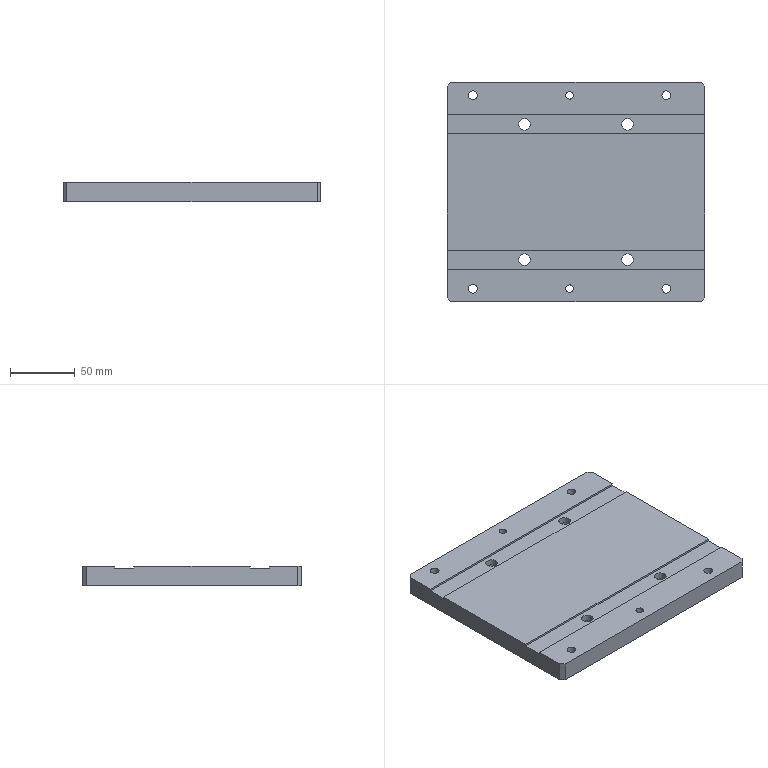Part | STEP file | 11-FGXW-07-0411 | 1 solid | 50 faces | box 200 x 170 x 15 mm | volume 490377 mm3 | cylinder 28 | plane 22 | commonest cylinder face diameters 6.8 x8 9 x8 15 x8 6 x4
STEP:
#1=CARTESIAN_POINT('',(47.5,52.5,8.6));
#2=VERTEX_POINT('',#1);
#3=CARTESIAN_POINT('',(32.5,52.5,8.6));
#4=VERTEX_POINT('',#3);
#5=CARTESIAN_POINT('',(40.,52.5,8.6));
#6=DIRECTION('',(0.,0.,-1.));
#7=DIRECTION('',(-1.,0.,0.));
#8=AXIS2_PLACEMENT_3D('',#5,#6,#7);
#9=CIRCLE('',#8,7.5);
#10=EDGE_CURVE('',#2,#4,#9,.T.);
#11=ORIENTED_EDGE('',*,*,#10,.F.);
#12=CARTESIAN_POINT('',(47.5,52.5,0.));
#13=VERTEX_POINT('',#12);
#14=CARTESIAN_POINT('',(47.5,52.5,0.));
#15=DIRECTION('',(0.,0.,-1.));
#16=VECTOR('',#15,1000.);
#17=LINE('',#14,#16);
#18=EDGE_CURVE('',#2,#13,#17,.T.);
#19=ORIENTED_EDGE('',*,*,#18,.T.);
#20=CARTESIAN_POINT('',(32.5,52.5,0.));
#21=VERTEX_POINT('',#20);
#22=CARTESIAN_POINT('',(40.,52.5,0.));
#23=DIRECTION('',(0.,0.,-1.));
#24=DIRECTION('',(-1.,0.,0.));
#25=AXIS2_PLACEMENT_3D('',#22,#23,#24);
#26=CIRCLE('',#25,7.5);
#27=EDGE_CURVE('',#13,#21,#26,.T.);
#28=ORIENTED_EDGE('',*,*,#27,.T.);
#29=CARTESIAN_POINT('',(32.5,52.5,0.));
#30=DIRECTION('',(0.,0.,-1.));
#31=VECTOR('',#30,1000.);
#32=LINE('',#29,#31);
#33=EDGE_CURVE('',#4,#21,#32,.T.);
#34=ORIENTED_EDGE('',*,*,#33,.F.);
#35=EDGE_LOOP('',(#11,#19,#28,#34));
#36=FACE_OUTER_BOUND('',#35,.T.);
#37=CARTESIAN_POINT('',(40.,52.5,0.));
#38=DIRECTION('',(0.,0.,-1.));
#39=DIRECTION('',(-1.,0.,0.));
#40=AXIS2_PLACEMENT_3D('',#37,#38,#39);
#41=CYLINDRICAL_SURFACE('',#40,7.5);
#42=ADVANCED_FACE('',(#36),#41,.F.);
#43=CARTESIAN_POINT('',(35.5,52.5,13.5));
#44=VERTEX_POINT('',#43);
#45=CARTESIAN_POINT('',(44.5,52.5,13.5));
#46=VERTEX_POINT('',#45);
#47=CARTESIAN_POINT('',(40.,52.5,13.5));
#48=DIRECTION('',(0.,0.,1.));
#49=DIRECTION('',(0.,1.,0.));
#50=AXIS2_PLACEMENT_3D('',#47,#48,#49);
#51=CIRCLE('',#50,4.5);
#52=EDGE_CURVE('',#44,#46,#51,.T.);
#53=ORIENTED_EDGE('',*,*,#52,.T.);
#54=CARTESIAN_POINT('',(44.5,52.5,8.6));
#55=VERTEX_POINT('',#54);
#56=CARTESIAN_POINT('',(44.5,52.5,0.));
#57=DIRECTION('',(0.,0.,-1.));
#58=VECTOR('',#57,1000.);
#59=LINE('',#56,#58);
#60=EDGE_CURVE('',#46,#55,#59,.T.);
#61=ORIENTED_EDGE('',*,*,#60,.T.);
#62=CARTESIAN_POINT('',(35.5,52.5,8.6));
#63=VERTEX_POINT('',#62);
#64=CARTESIAN_POINT('',(40.,52.5,8.6));
#65=DIRECTION('',(0.,0.,-1.));
#66=DIRECTION('',(-1.,0.,0.));
#67=AXIS2_PLACEMENT_3D('',#64,#65,#66);
#68=CIRCLE('',#67,4.5);
#69=EDGE_CURVE('',#55,#63,#68,.T.);
#70=ORIENTED_EDGE('',*,*,#69,.T.);
#71=CARTESIAN_POINT('',(35.5,52.5,0.));
#72=DIRECTION('',(0.,0.,-1.));
#73=VECTOR('',#72,1000.);
#74=LINE('',#71,#73);
#75=EDGE_CURVE('',#44,#63,#74,.T.);
#76=ORIENTED_EDGE('',*,*,#75,.F.);
#77=EDGE_LOOP('',(#53,#61,#70,#76));
#78=FACE_OUTER_BOUND('',#77,.T.);
#79=CARTESIAN_POINT('',(40.,52.5,0.));
#80=DIRECTION('',(0.,0.,-1.));
#81=DIRECTION('',(-1.,0.,0.));
#82=AXIS2_PLACEMENT_3D('',#79,#80,#81);
#83=CYLINDRICAL_SURFACE('',#82,4.5);
#84=ADVANCED_FACE('',(#78),#83,.F.);
#85=CARTESIAN_POINT('',(-32.5,52.5,8.6));
#86=VERTEX_POINT('',#85);
#87=CARTESIAN_POINT('',(-47.5,52.5,8.6));
#88=VERTEX_POINT('',#87);
#89=CARTESIAN_POINT('',(-40.,52.5,8.6));
#90=DIRECTION('',(0.,0.,-1.));
#91=DIRECTION('',(-1.,0.,0.));
#92=AXIS2_PLACEMENT_3D('',#89,#90,#91);
#93=CIRCLE('',#92,7.5);
#94=EDGE_CURVE('',#86,#88,#93,.T.);
#95=ORIENTED_EDGE('',*,*,#94,.F.);
#96=CARTESIAN_POINT('',(-32.5,52.5,0.));
#97=VERTEX_POINT('',#96);
#98=CARTESIAN_POINT('',(-32.5,52.5,0.));
#99=DIRECTION('',(0.,0.,-1.));
#100=VECTOR('',#99,1000.);
#101=LINE('',#98,#100);
#102=EDGE_CURVE('',#86,#97,#101,.T.);
#103=ORIENTED_EDGE('',*,*,#102,.T.);
#104=CARTESIAN_POINT('',(-47.5,52.5,0.));
#105=VERTEX_POINT('',#104);
#106=CARTESIAN_POINT('',(-40.,52.5,0.));
#107=DIRECTION('',(0.,0.,-1.));
#108=DIRECTION('',(-1.,0.,0.));
#109=AXIS2_PLACEMENT_3D('',#106,#107,#108);
#110=CIRCLE('',#109,7.5);
#111=EDGE_CURVE('',#97,#105,#110,.T.);
#112=ORIENTED_EDGE('',*,*,#111,.T.);
#113=CARTESIAN_POINT('',(-47.5,52.5,0.));
#114=DIRECTION('',(0.,0.,-1.));
#115=VECTOR('',#114,1000.);
#116=LINE('',#113,#115);
#117=EDGE_CURVE('',#88,#105,#116,.T.);
#118=ORIENTED_EDGE('',*,*,#117,.F.);
#119=EDGE_LOOP('',(#95,#103,#112,#118));
#120=FACE_OUTER_BOUND('',#119,.T.);
#121=CARTESIAN_POINT('',(-40.,52.5,0.));
#122=DIRECTION('',(0.,0.,-1.));
#123=DIRECTION('',(-1.,0.,0.));
#124=AXIS2_PLACEMENT_3D('',#121,#122,#123);
#125=CYLINDRICAL_SURFACE('',#124,7.5);
#126=ADVANCED_FACE('',(#120),#125,.F.);
#127=CARTESIAN_POINT('',(-44.5,52.5,13.5));
#128=VERTEX_POINT('',#127);
#129=CARTESIAN_POINT('',(-35.5,52.5,13.5));
#130=VERTEX_POINT('',#129);
#131=CARTESIAN_POINT('',(-40.,52.5,13.5));
#132=DIRECTION('',(0.,0.,1.));
#133=DIRECTION('',(0.,1.,0.));
#134=AXIS2_PLACEMENT_3D('',#131,#132,#133);
#135=CIRCLE('',#134,4.5);
#136=EDGE_CURVE('',#128,#130,#135,.T.);
#137=ORIENTED_EDGE('',*,*,#136,.T.);
#138=CARTESIAN_POINT('',(-35.5,52.5,8.6));
#139=VERTEX_POINT('',#138);
#140=CARTESIAN_POINT('',(-35.5,52.5,0.));
#141=DIRECTION('',(0.,0.,-1.));
#142=VECTOR('',#141,1000.);
#143=LINE('',#140,#142);
#144=EDGE_CURVE('',#130,#139,#143,.T.);
#145=ORIENTED_EDGE('',*,*,#144,.T.);
#146=CARTESIAN_POINT('',(-44.5,52.5,8.6));
#147=VERTEX_POINT('',#146);
#148=CARTESIAN_POINT('',(-40.,52.5,8.6));
#149=DIRECTION('',(0.,0.,-1.));
#150=DIRECTION('',(-1.,0.,0.));
#151=AXIS2_PLACEMENT_3D('',#148,#149,#150);
#152=CIRCLE('',#151,4.5);
#153=EDGE_CURVE('',#139,#147,#152,.T.);
#154=ORIENTED_EDGE('',*,*,#153,.T.);
#155=CARTESIAN_POINT('',(-44.5,52.5,0.));
#156=DIRECTION('',(0.,0.,-1.));
#157=VECTOR('',#156,1000.);
#158=LINE('',#155,#157);
#159=EDGE_CURVE('',#128,#147,#158,.T.);
#160=ORIENTED_EDGE('',*,*,#159,.F.);
#161=EDGE_LOOP('',(#137,#145,#154,#160));
#162=FACE_OUTER_BOUND('',#161,.T.);
#163=CARTESIAN_POINT('',(-40.,52.5,0.));
#164=DIRECTION('',(0.,0.,-1.));
#165=DIRECTION('',(-1.,0.,0.));
#166=AXIS2_PLACEMENT_3D('',#163,#164,#165);
#167=CYLINDRICAL_SURFACE('',#166,4.5);
#168=ADVANCED_FACE('',(#162),#167,.F.);
#169=CARTESIAN_POINT('',(-32.5,-52.5,8.6));
#170=VERTEX_POINT('',#169);
#171=CARTESIAN_POINT('',(-47.5,-52.5,8.6));
#172=VERTEX_POINT('',#171);
#173=CARTESIAN_POINT('',(-40.,-52.5,8.6));
#174=DIRECTION('',(0.,0.,-1.));
#175=DIRECTION('',(-1.,0.,0.));
#176=AXIS2_PLACEMENT_3D('',#173,#174,#175);
#177=CIRCLE('',#176,7.5);
#178=EDGE_CURVE('',#170,#172,#177,.T.);
#179=ORIENTED_EDGE('',*,*,#178,.F.);
#180=CARTESIAN_POINT('',(-32.5,-52.5,0.));
#181=VERTEX_POINT('',#180);
#182=CARTESIAN_POINT('',(-32.5,-52.5,0.));
#183=DIRECTION('',(0.,0.,-1.));
#184=VECTOR('',#183,1000.);
#185=LINE('',#182,#184);
#186=EDGE_CURVE('',#170,#181,#185,.T.);
#187=ORIENTED_EDGE('',*,*,#186,.T.);
#188=CARTESIAN_POINT('',(-47.5,-52.5,0.));
#189=VERTEX_POINT('',#188);
#190=CARTESIAN_POINT('',(-40.,-52.5,0.));
#191=DIRECTION('',(0.,0.,-1.));
#192=DIRECTION('',(-1.,0.,0.));
#193=AXIS2_PLACEMENT_3D('',#190,#191,#192);
#194=CIRCLE('',#193,7.5);
#195=EDGE_CURVE('',#181,#189,#194,.T.);
#196=ORIENTED_EDGE('',*,*,#195,.T.);
#197=CARTESIAN_POINT('',(-47.5,-52.5,0.));
#198=DIRECTION('',(0.,0.,-1.));
#199=VECTOR('',#198,1000.);
#200=LINE('',#197,#199);
#201=EDGE_CURVE('',#172,#189,#200,.T.);
#202=ORIENTED_EDGE('',*,*,#201,.F.);
#203=EDGE_LOOP('',(#179,#187,#196,#202));
#204=FACE_OUTER_BOUND('',#203,.T.);
#205=CARTESIAN_POINT('',(-40.,-52.5,0.));
#206=DIRECTION('',(0.,0.,-1.));
#207=DIRECTION('',(-1.,0.,0.));
#208=AXIS2_PLACEMENT_3D('',#205,#206,#207);
#209=CYLINDRICAL_SURFACE('',#208,7.5);
#210=ADVANCED_FACE('',(#204),#209,.F.);
#211=CARTESIAN_POINT('',(-44.5,-52.5,13.5));
#212=VERTEX_POINT('',#211);
#213=CARTESIAN_POINT('',(-35.5,-52.5,13.5));
#214=VERTEX_POINT('',#213);
#215=CARTESIAN_POINT('',(-40.,-52.5,13.5));
#216=DIRECTION('',(0.,0.,1.));
#217=DIRECTION('',(0.,1.,0.));
#218=AXIS2_PLACEMENT_3D('',#215,#216,#217);
#219=CIRCLE('',#218,4.5);
#220=EDGE_CURVE('',#212,#214,#219,.T.);
#221=ORIENTED_EDGE('',*,*,#220,.T.);
#222=CARTESIAN_POINT('',(-35.5,-52.5,8.6));
#223=VERTEX_POINT('',#222);
#224=CARTESIAN_POINT('',(-35.5,-52.5,0.));
#225=DIRECTION('',(0.,0.,-1.));
#226=VECTOR('',#225,1000.);
#227=LINE('',#224,#226);
#228=EDGE_CURVE('',#214,#223,#227,.T.);
#229=ORIENTED_EDGE('',*,*,#228,.T.);
#230=CARTESIAN_POINT('',(-44.5,-52.5,8.6));
#231=VERTEX_POINT('',#230);
#232=CARTESIAN_POINT('',(-40.,-52.5,8.6));
#233=DIRECTION('',(0.,0.,-1.));
#234=DIRECTION('',(-1.,0.,0.));
#235=AXIS2_PLACEMENT_3D('',#232,#233,#234);
#236=CIRCLE('',#235,4.5);
#237=EDGE_CURVE('',#223,#231,#236,.T.);
#238=ORIENTED_EDGE('',*,*,#237,.T.);
#239=CARTESIAN_POINT('',(-44.5,-52.5,0.));
#240=DIRECTION('',(0.,0.,-1.));
#241=VECTOR('',#240,1000.);
#242=LINE('',#239,#241);
#243=EDGE_CURVE('',#212,#231,#242,.T.);
#244=ORIENTED_EDGE('',*,*,#243,.F.);
#245=EDGE_LOOP('',(#221,#229,#238,#244));
#246=FACE_OUTER_BOUND('',#245,.T.);
#247=CARTESIAN_POINT('',(-40.,-52.5,0.));
#248=DIRECTION('',(0.,0.,-1.));
#249=DIRECTION('',(-1.,0.,0.));
#250=AXIS2_PLACEMENT_3D('',#247,#248,#249);
#251=CYLINDRICAL_SURFACE('',#250,4.5);
#252=ADVANCED_FACE('',(#246),#251,.F.);
#253=CARTESIAN_POINT('',(47.5,-52.5,8.6));
#254=VERTEX_POINT('',#253);
#255=CARTESIAN_POINT('',(32.5,-52.5,8.6));
#256=VERTEX_POINT('',#255);
#257=CARTESIAN_POINT('',(40.,-52.5,8.6));
#258=DIRECTION('',(0.,0.,-1.));
#259=DIRECTION('',(-1.,0.,0.));
#260=AXIS2_PLACEMENT_3D('',#257,#258,#259);
#261=CIRCLE('',#260,7.5);
#262=EDGE_CURVE('',#254,#256,#261,.T.);
#263=ORIENTED_EDGE('',*,*,#262,.F.);
#264=CARTESIAN_POINT('',(47.5,-52.5,0.));
#265=VERTEX_POINT('',#264);
#266=CARTESIAN_POINT('',(47.5,-52.5,0.));
#267=DIRECTION('',(0.,0.,-1.));
#268=VECTOR('',#267,1000.);
#269=LINE('',#266,#268);
#270=EDGE_CURVE('',#254,#265,#269,.T.);
#271=ORIENTED_EDGE('',*,*,#270,.T.);
#272=CARTESIAN_POINT('',(32.5,-52.5,0.));
#273=VERTEX_POINT('',#272);
#274=CARTESIAN_POINT('',(40.,-52.5,0.));
#275=DIRECTION('',(0.,0.,-1.));
#276=DIRECTION('',(-1.,0.,0.));
#277=AXIS2_PLACEMENT_3D('',#274,#275,#276);
#278=CIRCLE('',#277,7.5);
#279=EDGE_CURVE('',#265,#273,#278,.T.);
#280=ORIENTED_EDGE('',*,*,#279,.T.);
#281=CARTESIAN_POINT('',(32.5,-52.5,0.));
#282=DIRECTION('',(0.,0.,-1.));
#283=VECTOR('',#282,1000.);
#284=LINE('',#281,#283);
#285=EDGE_CURVE('',#256,#273,#284,.T.);
#286=ORIENTED_EDGE('',*,*,#285,.F.);
#287=EDGE_LOOP('',(#263,#271,#280,#286));
#288=FACE_OUTER_BOUND('',#287,.T.);
#289=CARTESIAN_POINT('',(40.,-52.5,0.));
#290=DIRECTION('',(0.,0.,-1.));
#291=DIRECTION('',(-1.,0.,0.));
#292=AXIS2_PLACEMENT_3D('',#289,#290,#291);
#293=CYLINDRICAL_SURFACE('',#292,7.5);
#294=ADVANCED_FACE('',(#288),#293,.F.);
#295=CARTESIAN_POINT('',(35.5,-52.5,13.5));
#296=VERTEX_POINT('',#295);
#297=CARTESIAN_POINT('',(44.5,-52.5,13.5));
#298=VERTEX_POINT('',#297);
#299=CARTESIAN_POINT('',(40.,-52.5,13.5));
#300=DIRECTION('',(0.,0.,1.));
#301=DIRECTION('',(0.,1.,0.));
#302=AXIS2_PLACEMENT_3D('',#299,#300,#301);
#303=CIRCLE('',#302,4.5);
#304=EDGE_CURVE('',#296,#298,#303,.T.);
#305=ORIENTED_EDGE('',*,*,#304,.T.);
#306=CARTESIAN_POINT('',(44.5,-52.5,8.6));
#307=VERTEX_POINT('',#306);
#308=CARTESIAN_POINT('',(44.5,-52.5,0.));
#309=DIRECTION('',(0.,0.,-1.));
#310=VECTOR('',#309,1000.);
#311=LINE('',#308,#310);
#312=EDGE_CURVE('',#298,#307,#311,.T.);
#313=ORIENTED_EDGE('',*,*,#312,.T.);
#314=CARTESIAN_POINT('',(35.5,-52.5,8.6));
#315=VERTEX_POINT('',#314);
#316=CARTESIAN_POINT('',(40.,-52.5,8.6));
#317=DIRECTION('',(0.,0.,-1.));
#318=DIRECTION('',(-1.,0.,0.));
#319=AXIS2_PLACEMENT_3D('',#316,#317,#318);
#320=CIRCLE('',#319,4.5);
#321=EDGE_CURVE('',#307,#315,#320,.T.);
#322=ORIENTED_EDGE('',*,*,#321,.T.);
#323=CARTESIAN_POINT('',(35.5,-52.5,0.));
#324=DIRECTION('',(0.,0.,-1.));
#325=VECTOR('',#324,1000.);
#326=LINE('',#323,#325);
#327=EDGE_CURVE('',#296,#315,#326,.T.);
#328=ORIENTED_EDGE('',*,*,#327,.F.);
#329=EDGE_LOOP('',(#305,#313,#322,#328));
#330=FACE_OUTER_BOUND('',#329,.T.);
#331=CARTESIAN_POINT('',(40.,-52.5,0.));
#332=DIRECTION('',(0.,0.,-1.));
#333=DIRECTION('',(-1.,0.,0.));
#334=AXIS2_PLACEMENT_3D('',#331,#332,#333);
#335=CYLINDRICAL_SURFACE('',#334,4.5);
#336=ADVANCED_FACE('',(#330),#335,.F.);
#337=CARTESIAN_POINT('',(-2.,-75.,15.));
#338=VERTEX_POINT('',#337);
#339=CARTESIAN_POINT('',(-8.,-75.,15.));
#340=VERTEX_POINT('',#339);
#341=CARTESIAN_POINT('',(-5.,-75.,15.));
#342=DIRECTION('',(0.,0.,-1.));
#343=DIRECTION('',(-1.,0.,0.));
#344=AXIS2_PLACEMENT_3D('',#341,#342,#343);
#345=CIRCLE('',#344,3.);
#346=EDGE_CURVE('',#338,#340,#345,.T.);
#347=ORIENTED_EDGE('',*,*,#346,.F.);
#348=CARTESIAN_POINT('',(-2.,-75.,0.));
#349=VERTEX_POINT('',#348);
#350=CARTESIAN_POINT('',(-2.,-75.,0.));
#351=DIRECTION('',(0.,0.,-1.));
#352=VECTOR('',#351,1000.);
#353=LINE('',#350,#352);
#354=EDGE_CURVE('',#338,#349,#353,.T.);
#355=ORIENTED_EDGE('',*,*,#354,.T.);
#356=CARTESIAN_POINT('',(-8.,-75.,0.));
#357=VERTEX_POINT('',#356);
#358=CARTESIAN_POINT('',(-5.,-75.,0.));
#359=DIRECTION('',(0.,0.,-1.));
#360=DIRECTION('',(-1.,0.,0.));
#361=AXIS2_PLACEMENT_3D('',#358,#359,#360);
#362=CIRCLE('',#361,3.);
#363=EDGE_CURVE('',#349,#357,#362,.T.);
#364=ORIENTED_EDGE('',*,*,#363,.T.);
#365=CARTESIAN_POINT('',(-8.,-75.,0.));
#366=DIRECTION('',(0.,0.,-1.));
#367=VECTOR('',#366,1000.);
#368=LINE('',#365,#367);
#369=EDGE_CURVE('',#340,#357,#368,.T.);
#370=ORIENTED_EDGE('',*,*,#369,.F.);
#371=EDGE_LOOP('',(#347,#355,#364,#370));
#372=FACE_OUTER_BOUND('',#371,.T.);
#373=CARTESIAN_POINT('',(-5.,-75.,0.));
#374=DIRECTION('',(0.,0.,-1.));
#375=DIRECTION('',(-1.,0.,0.));
#376=AXIS2_PLACEMENT_3D('',#373,#374,#375);
#377=CYLINDRICAL_SURFACE('',#376,3.);
#378=ADVANCED_FACE('',(#372),#377,.F.);
#379=CARTESIAN_POINT('',(-2.,75.,15.));
#380=VERTEX_POINT('',#379);
#381=CARTESIAN_POINT('',(-8.,75.,15.));
#382=VERTEX_POINT('',#381);
#383=CARTESIAN_POINT('',(-5.,75.,15.));
#384=DIRECTION('',(0.,0.,-1.));
#385=DIRECTION('',(-1.,0.,0.));
#386=AXIS2_PLACEMENT_3D('',#383,#384,#385);
#387=CIRCLE('',#386,3.);
#388=EDGE_CURVE('',#380,#382,#387,.T.);
#389=ORIENTED_EDGE('',*,*,#388,.F.);
#390=CARTESIAN_POINT('',(-2.,75.,0.));
#391=VERTEX_POINT('',#390);
#392=CARTESIAN_POINT('',(-2.,75.,0.));
#393=DIRECTION('',(0.,0.,-1.));
#394=VECTOR('',#393,1000.);
#395=LINE('',#392,#394);
#396=EDGE_CURVE('',#380,#391,#395,.T.);
#397=ORIENTED_EDGE('',*,*,#396,.T.);
#398=CARTESIAN_POINT('',(-8.,75.,0.));
#399=VERTEX_POINT('',#398);
#400=CARTESIAN_POINT('',(-5.,75.,0.));
#401=DIRECTION('',(0.,0.,-1.));
#402=DIRECTION('',(-1.,0.,0.));
#403=AXIS2_PLACEMENT_3D('',#400,#401,#402);
#404=CIRCLE('',#403,3.);
#405=EDGE_CURVE('',#391,#399,#404,.T.);
#406=ORIENTED_EDGE('',*,*,#405,.T.);
#407=CARTESIAN_POINT('',(-8.,75.,0.));
#408=DIRECTION('',(0.,0.,-1.));
#409=VECTOR('',#408,1000.);
#410=LINE('',#407,#409);
#411=EDGE_CURVE('',#382,#399,#410,.T.);
#412=ORIENTED_EDGE('',*,*,#411,.F.);
#413=EDGE_LOOP('',(#389,#397,#406,#412));
#414=FACE_OUTER_BOUND('',#413,.T.);
#415=CARTESIAN_POINT('',(-5.,75.,0.));
#416=DIRECTION('',(0.,0.,-1.));
#417=DIRECTION('',(-1.,0.,0.));
#418=AXIS2_PLACEMENT_3D('',#415,#416,#417);
#419=CYLINDRICAL_SURFACE('',#418,3.);
#420=ADVANCED_FACE('',(#414),#419,.F.);
#421=CARTESIAN_POINT('',(-76.6,75.,15.));
#422=VERTEX_POINT('',#421);
#423=CARTESIAN_POINT('',(-83.4,75.,15.));
#424=VERTEX_POINT('',#423);
#425=CARTESIAN_POINT('',(-80.,75.,15.));
#426=DIRECTION('',(0.,0.,-1.));
#427=DIRECTION('',(-1.,0.,0.));
#428=AXIS2_PLACEMENT_3D('',#425,#426,#427);
#429=CIRCLE('',#428,3.4);
#430=EDGE_CURVE('',#422,#424,#429,.T.);
#431=ORIENTED_EDGE('',*,*,#430,.F.);
#432=CARTESIAN_POINT('',(-76.6,75.,0.));
#433=VERTEX_POINT('',#432);
#434=CARTESIAN_POINT('',(-76.6,75.,0.));
#435=DIRECTION('',(0.,0.,-1.));
#436=VECTOR('',#435,1000.);
#437=LINE('',#434,#436);
#438=EDGE_CURVE('',#422,#433,#437,.T.);
#439=ORIENTED_EDGE('',*,*,#438,.T.);
#440=CARTESIAN_POINT('',(-83.4,75.,0.));
#441=VERTEX_POINT('',#440);
#442=CARTESIAN_POINT('',(-80.,75.,0.));
#443=DIRECTION('',(0.,0.,-1.));
#444=DIRECTION('',(-1.,0.,0.));
#445=AXIS2_PLACEMENT_3D('',#442,#443,#444);
#446=CIRCLE('',#445,3.4);
#447=EDGE_CURVE('',#433,#441,#446,.T.);
#448=ORIENTED_EDGE('',*,*,#447,.T.);
#449=CARTESIAN_POINT('',(-83.4,75.,0.));
#450=DIRECTION('',(0.,0.,-1.));
#451=VECTOR('',#450,1000.);
#452=LINE('',#449,#451);
#453=EDGE_CURVE('',#424,#441,#452,.T.);
#454=ORIENTED_EDGE('',*,*,#453,.F.);
#455=EDGE_LOOP('',(#431,#439,#448,#454));
#456=FACE_OUTER_BOUND('',#455,.T.);
#457=CARTESIAN_POINT('',(-80.,75.,0.));
#458=DIRECTION('',(0.,0.,-1.));
#459=DIRECTION('',(-1.,0.,0.));
#460=AXIS2_PLACEMENT_3D('',#457,#458,#459);
#461=CYLINDRICAL_SURFACE('',#460,3.4);
#462=ADVANCED_FACE('',(#456),#461,.F.);
#463=CARTESIAN_POINT('',(73.4,75.,15.));
#464=VERTEX_POINT('',#463);
#465=CARTESIAN_POINT('',(66.6,75.,15.));
#466=VERTEX_POINT('',#465);
#467=CARTESIAN_POINT('',(70.,75.,15.));
#468=DIRECTION('',(0.,0.,-1.));
#469=DIRECTION('',(-1.,0.,0.));
#470=AXIS2_PLACEMENT_3D('',#467,#468,#469);
#471=CIRCLE('',#470,3.4);
#472=EDGE_CURVE('',#464,#466,#471,.T.);
#473=ORIENTED_EDGE('',*,*,#472,.F.);
#474=CARTESIAN_POINT('',(73.4,75.,0.));
#475=VERTEX_POINT('',#474);
#476=CARTESIAN_POINT('',(73.4,75.,0.));
#477=DIRECTION('',(0.,0.,-1.));
#478=VECTOR('',#477,1000.);
#479=LINE('',#476,#478);
#480=EDGE_CURVE('',#464,#475,#479,.T.);
#481=ORIENTED_EDGE('',*,*,#480,.T.);
#482=CARTESIAN_POINT('',(66.6,75.,0.));
#483=VERTEX_POINT('',#482);
#484=CARTESIAN_POINT('',(70.,75.,0.));
#485=DIRECTION('',(0.,0.,-1.));
#486=DIRECTION('',(-1.,0.,0.));
#487=AXIS2_PLACEMENT_3D('',#484,#485,#486);
#488=CIRCLE('',#487,3.4);
#489=EDGE_CURVE('',#475,#483,#488,.T.);
#490=ORIENTED_EDGE('',*,*,#489,.T.);
#491=CARTESIAN_POINT('',(66.6,75.,0.));
#492=DIRECTION('',(0.,0.,-1.));
#493=VECTOR('',#492,1000.);
#494=LINE('',#491,#493);
#495=EDGE_CURVE('',#466,#483,#494,.T.);
#496=ORIENTED_EDGE('',*,*,#495,.F.);
#497=EDGE_LOOP('',(#473,#481,#490,#496));
#498=FACE_OUTER_BOUND('',#497,.T.);
#499=CARTESIAN_POINT('',(70.,75.,0.));
#500=DIRECTION('',(0.,0.,-1.));
#501=DIRECTION('',(-1.,0.,0.));
#502=AXIS2_PLACEMENT_3D('',#499,#500,#501);
#503=CYLINDRICAL_SURFACE('',#502,3.4);
#504=ADVANCED_FACE('',(#498),#503,.F.);
#505=CARTESIAN_POINT('',(73.4,-75.,15.));
#506=VERTEX_POINT('',#505);
#507=CARTESIAN_POINT('',(66.6,-75.,15.));
#508=VERTEX_POINT('',#507);
#509=CARTESIAN_POINT('',(70.,-75.,15.));
#510=DIRECTION('',(0.,0.,-1.));
#511=DIRECTION('',(-1.,0.,0.));
#512=AXIS2_PLACEMENT_3D('',#509,#510,#511);
#513=CIRCLE('',#512,3.4);
#514=EDGE_CURVE('',#506,#508,#513,.T.);
#515=ORIENTED_EDGE('',*,*,#514,.F.);
#516=CARTESIAN_POINT('',(73.4,-75.,0.));
#517=VERTEX_POINT('',#516);
#518=CARTESIAN_POINT('',(73.4,-75.,0.));
#519=DIRECTION('',(0.,0.,-1.));
#520=VECTOR('',#519,1000.);
#521=LINE('',#518,#520);
#522=EDGE_CURVE('',#506,#517,#521,.T.);
#523=ORIENTED_EDGE('',*,*,#522,.T.);
#524=CARTESIAN_POINT('',(66.6,-75.,0.));
#525=VERTEX_POINT('',#524);
#526=CARTESIAN_POINT('',(70.,-75.,0.));
#527=DIRECTION('',(0.,0.,-1.));
#528=DIRECTION('',(-1.,0.,0.));
#529=AXIS2_PLACEMENT_3D('',#526,#527,#528);
#530=CIRCLE('',#529,3.4);
#531=EDGE_CURVE('',#517,#525,#530,.T.);
#532=ORIENTED_EDGE('',*,*,#531,.T.);
#533=CARTESIAN_POINT('',(66.6,-75.,0.));
#534=DIRECTION('',(0.,0.,-1.));
#535=VECTOR('',#534,1000.);
#536=LINE('',#533,#535);
#537=EDGE_CURVE('',#508,#525,#536,.T.);
#538=ORIENTED_EDGE('',*,*,#537,.F.);
#539=EDGE_LOOP('',(#515,#523,#532,#538));
#540=FACE_OUTER_BOUND('',#539,.T.);
#541=CARTESIAN_POINT('',(70.,-75.,0.));
#542=DIRECTION('',(0.,0.,-1.));
#543=DIRECTION('',(-1.,0.,0.));
#544=AXIS2_PLACEMENT_3D('',#541,#542,#543);
#545=CYLINDRICAL_SURFACE('',#544,3.4);
#546=ADVANCED_FACE('',(#540),#545,.F.);
#547=CARTESIAN_POINT('',(-76.6,-75.,15.));
#548=VERTEX_POINT('',#547);
#549=CARTESIAN_POINT('',(-83.4,-75.,15.));
#550=VERTEX_POINT('',#549);
#551=CARTESIAN_POINT('',(-80.,-75.,15.));
#552=DIRECTION('',(0.,0.,-1.));
#553=DIRECTION('',(-1.,0.,0.));
#554=AXIS2_PLACEMENT_3D('',#551,#552,#553);
#555=CIRCLE('',#554,3.4);
#556=EDGE_CURVE('',#548,#550,#555,.T.);
#557=ORIENTED_EDGE('',*,*,#556,.F.);
#558=CARTESIAN_POINT('',(-76.6,-75.,0.));
#559=VERTEX_POINT('',#558);
#560=CARTESIAN_POINT('',(-76.6,-75.,0.));
#561=DIRECTION('',(0.,0.,-1.));
#562=VECTOR('',#561,1000.);
#563=LINE('',#560,#562);
#564=EDGE_CURVE('',#548,#559,#563,.T.);
#565=ORIENTED_EDGE('',*,*,#564,.T.);
#566=CARTESIAN_POINT('',(-83.4,-75.,0.));
#567=VERTEX_POINT('',#566);
#568=CARTESIAN_POINT('',(-80.,-75.,0.));
#569=DIRECTION('',(0.,0.,-1.));
#570=DIRECTION('',(-1.,0.,0.));
#571=AXIS2_PLACEMENT_3D('',#568,#569,#570);
#572=CIRCLE('',#571,3.4);
#573=EDGE_CURVE('',#559,#567,#572,.T.);
#574=ORIENTED_EDGE('',*,*,#573,.T.);
#575=CARTESIAN_POINT('',(-83.4,-75.,0.));
#576=DIRECTION('',(0.,0.,-1.));
#577=VECTOR('',#576,1000.);
#578=LINE('',#575,#577);
#579=EDGE_CURVE('',#550,#567,#578,.T.);
#580=ORIENTED_EDGE('',*,*,#579,.F.);
#581=EDGE_LOOP('',(#557,#565,#574,#580));
#582=FACE_OUTER_BOUND('',#581,.T.);
#583=CARTESIAN_POINT('',(-80.,-75.,0.));
#584=DIRECTION('',(0.,0.,-1.));
#585=DIRECTION('',(-1.,0.,0.));
#586=AXIS2_PLACEMENT_3D('',#583,#584,#585);
#587=CYLINDRICAL_SURFACE('',#586,3.4);
#588=ADVANCED_FACE('',(#582),#587,.F.);
#589=CARTESIAN_POINT('',(-5.,-75.,15.));
#590=DIRECTION('',(0.,0.,-1.));
#591=DIRECTION('',(-1.,0.,0.));
#592=AXIS2_PLACEMENT_3D('',#589,#590,#591);
#593=CIRCLE('',#592,3.);
#594=EDGE_CURVE('',#340,#338,#593,.T.);
#595=ORIENTED_EDGE('',*,*,#594,.T.);
#596=ORIENTED_EDGE('',*,*,#346,.T.);
#597=EDGE_LOOP('',(#595,#596));
#598=FACE_BOUND('',#597,.T.);
#599=CARTESIAN_POINT('',(70.,-75.,15.));
#600=DIRECTION('',(0.,0.,-1.));
#601=DIRECTION('',(-1.,0.,0.));
#602=AXIS2_PLACEMENT_3D('',#599,#600,#601);
#603=CIRCLE('',#602,3.4);
#604=EDGE_CURVE('',#508,#506,#603,.T.);
#605=ORIENTED_EDGE('',*,*,#604,.T.);
#606=ORIENTED_EDGE('',*,*,#514,.T.);
#607=EDGE_LOOP('',(#605,#606));
#608=FACE_BOUND('',#607,.T.);
#609=CARTESIAN_POINT('',(-80.,-75.,15.));
#610=DIRECTION('',(0.,0.,-1.));
#611=DIRECTION('',(-1.,0.,0.));
#612=AXIS2_PLACEMENT_3D('',#609,#610,#611);
#613=CIRCLE('',#612,3.4);
#614=EDGE_CURVE('',#550,#548,#613,.T.);
#615=ORIENTED_EDGE('',*,*,#614,.T.);
#616=ORIENTED_EDGE('',*,*,#556,.T.);
#617=EDGE_LOOP('',(#615,#616));
#618=FACE_BOUND('',#617,.T.);
#619=CARTESIAN_POINT('',(100.,-82.,15.));
#620=VERTEX_POINT('',#619);
#621=CARTESIAN_POINT('',(100.,-60.,15.));
#622=VERTEX_POINT('',#621);
#623=CARTESIAN_POINT('',(100.,-85.,15.));
#624=DIRECTION('',(0.,1.,0.));
#625=VECTOR('',#624,1000.);
#626=LINE('',#623,#625);
#627=EDGE_CURVE('',#620,#622,#626,.T.);
#628=ORIENTED_EDGE('',*,*,#627,.T.);
#629=CARTESIAN_POINT('',(-100.,-60.,15.));
#630=VERTEX_POINT('',#629);
#631=CARTESIAN_POINT('',(100.,-60.,15.));
#632=DIRECTION('',(-1.,0.,0.));
#633=VECTOR('',#632,1000.);
#634=LINE('',#631,#633);
#635=EDGE_CURVE('',#622,#630,#634,.T.);
#636=ORIENTED_EDGE('',*,*,#635,.T.);
#637=CARTESIAN_POINT('',(-100.,-82.,15.));
#638=VERTEX_POINT('',#637);
#639=CARTESIAN_POINT('',(-100.,-85.,15.));
#640=DIRECTION('',(0.,-1.,0.));
#641=VECTOR('',#640,1000.);
#642=LINE('',#639,#641);
#643=EDGE_CURVE('',#630,#638,#642,.T.);
#644=ORIENTED_EDGE('',*,*,#643,.T.);
#645=CARTESIAN_POINT('',(-97.,-85.,15.));
#646=VERTEX_POINT('',#645);
#647=CARTESIAN_POINT('',(-97.,-85.,15.));
#648=DIRECTION('',(0.7071,-0.7071,0.));
#649=VECTOR('',#648,1000.);
#650=LINE('',#647,#649);
#651=EDGE_CURVE('',#638,#646,#650,.T.);
#652=ORIENTED_EDGE('',*,*,#651,.T.);
#653=CARTESIAN_POINT('',(97.,-85.,15.));
#654=VERTEX_POINT('',#653);
#655=CARTESIAN_POINT('',(-100.,-85.,15.));
#656=DIRECTION('',(1.,0.,0.));
#657=VECTOR('',#656,1000.);
#658=LINE('',#655,#657);
#659=EDGE_CURVE('',#646,#654,#658,.T.);
#660=ORIENTED_EDGE('',*,*,#659,.T.);
#661=CARTESIAN_POINT('',(100.,-82.,15.));
#662=DIRECTION('',(0.7071,0.7071,0.));
#663=VECTOR('',#662,1000.);
#664=LINE('',#661,#663);
#665=EDGE_CURVE('',#654,#620,#664,.T.);
#666=ORIENTED_EDGE('',*,*,#665,.T.);
#667=EDGE_LOOP('',(#628,#636,#644,#652,#660,#666));
#668=FACE_OUTER_BOUND('',#667,.T.);
#669=CARTESIAN_POINT('',(0.,0.,15.));
#670=DIRECTION('',(0.,0.,-1.));
#671=DIRECTION('',(-1.,0.,0.));
#672=AXIS2_PLACEMENT_3D('',#669,#670,#671);
#673=PLANE('',#672);
#674=ADVANCED_FACE('',(#598,#608,#618,#668),#673,.F.);
#675=CARTESIAN_POINT('',(-100.,45.,15.));
#676=VERTEX_POINT('',#675);
#677=CARTESIAN_POINT('',(-100.,-45.,15.));
#678=VERTEX_POINT('',#677);
#679=CARTESIAN_POINT('',(-100.,-85.,15.));
#680=DIRECTION('',(0.,-1.,0.));
#681=VECTOR('',#680,1000.);
#682=LINE('',#679,#681);
#683=EDGE_CURVE('',#676,#678,#682,.T.);
#684=ORIENTED_EDGE('',*,*,#683,.T.);
#685=CARTESIAN_POINT('',(100.,-45.,15.));
#686=VERTEX_POINT('',#685);
#687=CARTESIAN_POINT('',(100.,-45.,15.));
#688=DIRECTION('',(-1.,0.,0.));
#689=VECTOR('',#688,1000.);
#690=LINE('',#687,#689);
#691=EDGE_CURVE('',#686,#678,#690,.T.);
#692=ORIENTED_EDGE('',*,*,#691,.F.);
#693=CARTESIAN_POINT('',(100.,45.,15.));
#694=VERTEX_POINT('',#693);
#695=CARTESIAN_POINT('',(100.,-85.,15.));
#696=DIRECTION('',(0.,1.,0.));
#697=VECTOR('',#696,1000.);
#698=LINE('',#695,#697);
#699=EDGE_CURVE('',#686,#694,#698,.T.);
#700=ORIENTED_EDGE('',*,*,#699,.T.);
#701=CARTESIAN_POINT('',(100.,45.,15.));
#702=DIRECTION('',(-1.,0.,0.));
#703=VECTOR('',#702,1000.);
#704=LINE('',#701,#703);
#705=EDGE_CURVE('',#694,#676,#704,.T.);
#706=ORIENTED_EDGE('',*,*,#705,.T.);
#707=EDGE_LOOP('',(#684,#692,#700,#706));
#708=FACE_OUTER_BOUND('',#707,.T.);
#709=CARTESIAN_POINT('',(0.,0.,15.));
#710=DIRECTION('',(0.,0.,-1.));
#711=DIRECTION('',(-1.,0.,0.));
#712=AXIS2_PLACEMENT_3D('',#709,#710,#711);
#713=PLANE('',#712);
#714=ADVANCED_FACE('',(#708),#713,.F.);
#715=CARTESIAN_POINT('',(100.,-45.,13.5));
#716=VERTEX_POINT('',#715);
#717=CARTESIAN_POINT('',(100.,-60.,13.5));
#718=VERTEX_POINT('',#717);
#719=CARTESIAN_POINT('',(100.,-45.,13.5));
#720=DIRECTION('',(0.,-1.,0.));
#721=VECTOR('',#720,1000.);
#722=LINE('',#719,#721);
#723=EDGE_CURVE('',#716,#718,#722,.T.);
#724=ORIENTED_EDGE('',*,*,#723,.T.);
#725=CARTESIAN_POINT('',(100.,-60.,15.));
#726=DIRECTION('',(0.,0.,1.));
#727=VECTOR('',#726,1000.);
#728=LINE('',#725,#727);
#729=EDGE_CURVE('',#718,#622,#728,.T.);
#730=ORIENTED_EDGE('',*,*,#729,.T.);
#731=ORIENTED_EDGE('',*,*,#627,.F.);
#732=CARTESIAN_POINT('',(100.,-82.,0.));
#733=VERTEX_POINT('',#732);
#734=CARTESIAN_POINT('',(100.,-82.,15.));
#735=DIRECTION('',(0.,0.,-1.));
#736=VECTOR('',#735,1000.);
#737=LINE('',#734,#736);
#738=EDGE_CURVE('',#620,#733,#737,.T.);
#739=ORIENTED_EDGE('',*,*,#738,.T.);
#740=CARTESIAN_POINT('',(100.,82.,0.));
#741=VERTEX_POINT('',#740);
#742=CARTESIAN_POINT('',(100.,-85.,0.));
#743=DIRECTION('',(0.,1.,0.));
#744=VECTOR('',#743,1000.);
#745=LINE('',#742,#744);
#746=EDGE_CURVE('',#733,#741,#745,.T.);
#747=ORIENTED_EDGE('',*,*,#746,.T.);
#748=CARTESIAN_POINT('',(100.,82.,15.));
#749=VERTEX_POINT('',#748);
#750=CARTESIAN_POINT('',(100.,82.,15.));
#751=DIRECTION('',(0.,0.,1.));
#752=VECTOR('',#751,1000.);
#753=LINE('',#750,#752);
#754=EDGE_CURVE('',#741,#749,#753,.T.);
#755=ORIENTED_EDGE('',*,*,#754,.T.);
#756=CARTESIAN_POINT('',(100.,60.,15.));
#757=VERTEX_POINT('',#756);
#758=CARTESIAN_POINT('',(100.,-85.,15.));
#759=DIRECTION('',(0.,1.,0.));
#760=VECTOR('',#759,1000.);
#761=LINE('',#758,#760);
#762=EDGE_CURVE('',#757,#749,#761,.T.);
#763=ORIENTED_EDGE('',*,*,#762,.F.);
#764=CARTESIAN_POINT('',(100.,60.,13.5));
#765=VERTEX_POINT('',#764);
#766=CARTESIAN_POINT('',(100.,60.,15.));
#767=DIRECTION('',(0.,0.,-1.));
#768=VECTOR('',#767,1000.);
#769=LINE('',#766,#768);
#770=EDGE_CURVE('',#757,#765,#769,.T.);
#771=ORIENTED_EDGE('',*,*,#770,.T.);
#772=CARTESIAN_POINT('',(100.,45.,13.5));
#773=VERTEX_POINT('',#772);
#774=CARTESIAN_POINT('',(100.,45.,13.5));
#775=DIRECTION('',(0.,-1.,0.));
#776=VECTOR('',#775,1000.);
#777=LINE('',#774,#776);
#778=EDGE_CURVE('',#765,#773,#777,.T.);
#779=ORIENTED_EDGE('',*,*,#778,.T.);
#780=CARTESIAN_POINT('',(100.,45.,15.));
#781=DIRECTION('',(0.,0.,1.));
#782=VECTOR('',#781,1000.);
#783=LINE('',#780,#782);
#784=EDGE_CURVE('',#773,#694,#783,.T.);
#785=ORIENTED_EDGE('',*,*,#784,.T.);
#786=ORIENTED_EDGE('',*,*,#699,.F.);
#787=CARTESIAN_POINT('',(100.,-45.,15.));
#788=DIRECTION('',(0.,0.,-1.));
#789=VECTOR('',#788,1000.);
#790=LINE('',#787,#789);
#791=EDGE_CURVE('',#686,#716,#790,.T.);
#792=ORIENTED_EDGE('',*,*,#791,.T.);
#793=EDGE_LOOP('',(#724,#730,#731,#739,#747,#755,#763,#771,#779,#785,#786,#792));
#794=FACE_OUTER_BOUND('',#793,.T.);
#795=CARTESIAN_POINT('',(100.,-85.,15.));
#796=DIRECTION('',(-1.,0.,0.));
#797=DIRECTION('',(0.,0.,1.));
#798=AXIS2_PLACEMENT_3D('',#795,#796,#797);
#799=PLANE('',#798);
#800=ADVANCED_FACE('',(#794),#799,.F.);
#801=CARTESIAN_POINT('',(97.,85.,0.));
#802=VERTEX_POINT('',#801);
#803=CARTESIAN_POINT('',(-97.,85.,0.));
#804=VERTEX_POINT('',#803);
#805=CARTESIAN_POINT('',(-100.,85.,0.));
#806=DIRECTION('',(-1.,0.,0.));
#807=VECTOR('',#806,1000.);
#808=LINE('',#805,#807);
#809=EDGE_CURVE('',#802,#804,#808,.T.);
#810=ORIENTED_EDGE('',*,*,#809,.T.);
#811=CARTESIAN_POINT('',(-97.,85.,15.));
#812=VERTEX_POINT('',#811);
#813=CARTESIAN_POINT('',(-97.,85.,15.));
#814=DIRECTION('',(0.,0.,1.));
#815=VECTOR('',#814,1000.);
#816=LINE('',#813,#815);
#817=EDGE_CURVE('',#804,#812,#816,.T.);
#818=ORIENTED_EDGE('',*,*,#817,.T.);
#819=CARTESIAN_POINT('',(97.,85.,15.));
#820=VERTEX_POINT('',#819);
#821=CARTESIAN_POINT('',(-100.,85.,15.));
#822=DIRECTION('',(-1.,0.,0.));
#823=VECTOR('',#822,1000.);
#824=LINE('',#821,#823);
#825=EDGE_CURVE('',#820,#812,#824,.T.);
#826=ORIENTED_EDGE('',*,*,#825,.F.);
#827=CARTESIAN_POINT('',(97.,85.,15.));
#828=DIRECTION('',(0.,0.,-1.));
#829=VECTOR('',#828,1000.);
#830=LINE('',#827,#829);
#831=EDGE_CURVE('',#820,#802,#830,.T.);
#832=ORIENTED_EDGE('',*,*,#831,.T.);
#833=EDGE_LOOP('',(#810,#818,#826,#832));
#834=FACE_OUTER_BOUND('',#833,.T.);
#835=CARTESIAN_POINT('',(-100.,85.,15.));
#836=DIRECTION('',(0.,-1.,0.));
#837=DIRECTION('',(0.,0.,-1.));
#838=AXIS2_PLACEMENT_3D('',#835,#836,#837);
#839=PLANE('',#838);
#840=ADVANCED_FACE('',(#834),#839,.F.);
#841=ORIENTED_EDGE('',*,*,#643,.F.);
#842=CARTESIAN_POINT('',(-100.,-60.,13.5));
#843=VERTEX_POINT('',#842);
#844=CARTESIAN_POINT('',(-100.,-60.,15.));
#845=DIRECTION('',(0.,0.,1.));
#846=VECTOR('',#845,1000.);
#847=LINE('',#844,#846);
#848=EDGE_CURVE('',#843,#630,#847,.T.);
#849=ORIENTED_EDGE('',*,*,#848,.F.);
#850=CARTESIAN_POINT('',(-100.,-45.,13.5));
#851=VERTEX_POINT('',#850);
#852=CARTESIAN_POINT('',(-100.,-45.,13.5));
#853=DIRECTION('',(0.,-1.,0.));
#854=VECTOR('',#853,1000.);
#855=LINE('',#852,#854);
#856=EDGE_CURVE('',#851,#843,#855,.T.);
#857=ORIENTED_EDGE('',*,*,#856,.F.);
#858=CARTESIAN_POINT('',(-100.,-45.,15.));
#859=DIRECTION('',(0.,0.,-1.));
#860=VECTOR('',#859,1000.);
#861=LINE('',#858,#860);
#862=EDGE_CURVE('',#678,#851,#861,.T.);
#863=ORIENTED_EDGE('',*,*,#862,.F.);
#864=ORIENTED_EDGE('',*,*,#683,.F.);
#865=CARTESIAN_POINT('',(-100.,45.,13.5));
#866=VERTEX_POINT('',#865);
#867=CARTESIAN_POINT('',(-100.,45.,15.));
#868=DIRECTION('',(0.,0.,1.));
#869=VECTOR('',#868,1000.);
#870=LINE('',#867,#869);
#871=EDGE_CURVE('',#866,#676,#870,.T.);
#872=ORIENTED_EDGE('',*,*,#871,.F.);
#873=CARTESIAN_POINT('',(-100.,60.,13.5));
#874=VERTEX_POINT('',#873);
#875=CARTESIAN_POINT('',(-100.,45.,13.5));
#876=DIRECTION('',(0.,-1.,0.));
#877=VECTOR('',#876,1000.);
#878=LINE('',#875,#877);
#879=EDGE_CURVE('',#874,#866,#878,.T.);
#880=ORIENTED_EDGE('',*,*,#879,.F.);
#881=CARTESIAN_POINT('',(-100.,60.,15.));
#882=VERTEX_POINT('',#881);
#883=CARTESIAN_POINT('',(-100.,60.,15.));
#884=DIRECTION('',(0.,0.,-1.));
#885=VECTOR('',#884,1000.);
#886=LINE('',#883,#885);
#887=EDGE_CURVE('',#882,#874,#886,.T.);
#888=ORIENTED_EDGE('',*,*,#887,.F.);
#889=CARTESIAN_POINT('',(-100.,82.,15.));
#890=VERTEX_POINT('',#889);
#891=CARTESIAN_POINT('',(-100.,-85.,15.));
#892=DIRECTION('',(0.,-1.,0.));
#893=VECTOR('',#892,1000.);
#894=LINE('',#891,#893);
#895=EDGE_CURVE('',#890,#882,#894,.T.);
#896=ORIENTED_EDGE('',*,*,#895,.F.);
#897=CARTESIAN_POINT('',(-100.,82.,0.));
#898=VERTEX_POINT('',#897);
#899=CARTESIAN_POINT('',(-100.,82.,15.));
#900=DIRECTION('',(0.,0.,-1.));
#901=VECTOR('',#900,1000.);
#902=LINE('',#899,#901);
#903=EDGE_CURVE('',#890,#898,#902,.T.);
#904=ORIENTED_EDGE('',*,*,#903,.T.);
#905=CARTESIAN_POINT('',(-100.,-82.,0.));
#906=VERTEX_POINT('',#905);
#907=CARTESIAN_POINT('',(-100.,-85.,0.));
#908=DIRECTION('',(0.,-1.,0.));
#909=VECTOR('',#908,1000.);
#910=LINE('',#907,#909);
#911=EDGE_CURVE('',#898,#906,#910,.T.);
#912=ORIENTED_EDGE('',*,*,#911,.T.);
#913=CARTESIAN_POINT('',(-100.,-82.,15.));
#914=DIRECTION('',(0.,0.,1.));
#915=VECTOR('',#914,1000.);
#916=LINE('',#913,#915);
#917=EDGE_CURVE('',#906,#638,#916,.T.);
#918=ORIENTED_EDGE('',*,*,#917,.T.);
#919=EDGE_LOOP('',(#841,#849,#857,#863,#864,#872,#880,#888,#896,#904,#912,#918));
#920=FACE_OUTER_BOUND('',#919,.T.);
#921=CARTESIAN_POINT('',(-100.,-85.,15.));
#922=DIRECTION('',(1.,0.,0.));
#923=DIRECTION('',(0.,0.,-1.));
#924=AXIS2_PLACEMENT_3D('',#921,#922,#923);
#925=PLANE('',#924);
#926=ADVANCED_FACE('',(#920),#925,.F.);
#927=ORIENTED_EDGE('',*,*,#659,.F.);
#928=CARTESIAN_POINT('',(-97.,-85.,0.));
#929=VERTEX_POINT('',#928);
#930=CARTESIAN_POINT('',(-97.,-85.,15.));
#931=DIRECTION('',(0.,0.,-1.));
#932=VECTOR('',#931,1000.);
#933=LINE('',#930,#932);
#934=EDGE_CURVE('',#646,#929,#933,.T.);
#935=ORIENTED_EDGE('',*,*,#934,.T.);
#936=CARTESIAN_POINT('',(97.,-85.,0.));
#937=VERTEX_POINT('',#936);
#938=CARTESIAN_POINT('',(-100.,-85.,0.));
#939=DIRECTION('',(1.,0.,0.));
#940=VECTOR('',#939,1000.);
#941=LINE('',#938,#940);
#942=EDGE_CURVE('',#929,#937,#941,.T.);
#943=ORIENTED_EDGE('',*,*,#942,.T.);
#944=CARTESIAN_POINT('',(97.,-85.,15.));
#945=DIRECTION('',(0.,0.,1.));
#946=VECTOR('',#945,1000.);
#947=LINE('',#944,#946);
#948=EDGE_CURVE('',#937,#654,#947,.T.);
#949=ORIENTED_EDGE('',*,*,#948,.T.);
#950=EDGE_LOOP('',(#927,#935,#943,#949));
#951=FACE_OUTER_BOUND('',#950,.T.);
#952=CARTESIAN_POINT('',(-100.,-85.,15.));
#953=DIRECTION('',(0.,1.,0.));
#954=DIRECTION('',(0.,0.,1.));
#955=AXIS2_PLACEMENT_3D('',#952,#953,#954);
#956=PLANE('',#955);
#957=ADVANCED_FACE('',(#951),#956,.F.);
#958=CARTESIAN_POINT('',(-5.,75.,15.));
#959=DIRECTION('',(0.,0.,-1.));
#960=DIRECTION('',(-1.,0.,0.));
#961=AXIS2_PLACEMENT_3D('',#958,#959,#960);
#962=CIRCLE('',#961,3.);
#963=EDGE_CURVE('',#382,#380,#962,.T.);
#964=ORIENTED_EDGE('',*,*,#963,.T.);
#965=ORIENTED_EDGE('',*,*,#388,.T.);
#966=EDGE_LOOP('',(#964,#965));
#967=FACE_BOUND('',#966,.T.);
#968=CARTESIAN_POINT('',(-80.,75.,15.));
#969=DIRECTION('',(0.,0.,-1.));
#970=DIRECTION('',(-1.,0.,0.));
#971=AXIS2_PLACEMENT_3D('',#968,#969,#970);
#972=CIRCLE('',#971,3.4);
#973=EDGE_CURVE('',#424,#422,#972,.T.);
#974=ORIENTED_EDGE('',*,*,#973,.T.);
#975=ORIENTED_EDGE('',*,*,#430,.T.);
#976=EDGE_LOOP('',(#974,#975));
#977=FACE_BOUND('',#976,.T.);
#978=CARTESIAN_POINT('',(70.,75.,15.));
#979=DIRECTION('',(0.,0.,-1.));
#980=DIRECTION('',(-1.,0.,0.));
#981=AXIS2_PLACEMENT_3D('',#978,#979,#980);
#982=CIRCLE('',#981,3.4);
#983=EDGE_CURVE('',#466,#464,#982,.T.);
#984=ORIENTED_EDGE('',*,*,#983,.T.);
#985=ORIENTED_EDGE('',*,*,#472,.T.);
#986=EDGE_LOOP('',(#984,#985));
#987=FACE_BOUND('',#986,.T.);
#988=ORIENTED_EDGE('',*,*,#895,.T.);
#989=CARTESIAN_POINT('',(100.,60.,15.));
#990=DIRECTION('',(-1.,0.,0.));
#991=VECTOR('',#990,1000.);
#992=LINE('',#989,#991);
#993=EDGE_CURVE('',#757,#882,#992,.T.);
#994=ORIENTED_EDGE('',*,*,#993,.F.);
#995=ORIENTED_EDGE('',*,*,#762,.T.);
#996=CARTESIAN_POINT('',(97.,85.,15.));
#997=DIRECTION('',(-0.7071,0.7071,0.));
#998=VECTOR('',#997,1000.);
#999=LINE('',#996,#998);
#1000=EDGE_CURVE('',#749,#820,#999,.T.);
#1001=ORIENTED_EDGE('',*,*,#1000,.T.);
#1002=ORIENTED_EDGE('',*,*,#825,.T.);
#1003=CARTESIAN_POINT('',(-100.,82.,15.));
#1004=DIRECTION('',(-0.7071,-0.7071,0.));
#1005=VECTOR('',#1004,1000.);
#1006=LINE('',#1003,#1005);
#1007=EDGE_CURVE('',#812,#890,#1006,.T.);
#1008=ORIENTED_EDGE('',*,*,#1007,.T.);
#1009=EDGE_LOOP('',(#988,#994,#995,#1001,#1002,#1008));
#1010=FACE_OUTER_BOUND('',#1009,.T.);
#1011=CARTESIAN_POINT('',(0.,0.,15.));
#1012=DIRECTION('',(0.,0.,-1.));
#1013=DIRECTION('',(-1.,0.,0.));
#1014=AXIS2_PLACEMENT_3D('',#1011,#1012,#1013);
#1015=PLANE('',#1014);
#1016=ADVANCED_FACE('',(#967,#977,#987,#1010),#1015,.F.);
#1017=CARTESIAN_POINT('',(40.,52.5,0.));
#1018=DIRECTION('',(0.,0.,-1.));
#1019=DIRECTION('',(-1.,0.,0.));
#1020=AXIS2_PLACEMENT_3D('',#1017,#1018,#1019);
#1021=CIRCLE('',#1020,7.5);
#1022=EDGE_CURVE('',#21,#13,#1021,.T.);
#1023=ORIENTED_EDGE('',*,*,#1022,.F.);
#1024=ORIENTED_EDGE('',*,*,#27,.F.);
#1025=EDGE_LOOP('',(#1023,#1024));
#1026=FACE_BOUND('',#1025,.T.);
#1027=CARTESIAN_POINT('',(-40.,52.5,0.));
#1028=DIRECTION('',(0.,0.,-1.));
#1029=DIRECTION('',(-1.,0.,0.));
#1030=AXIS2_PLACEMENT_3D('',#1027,#1028,#1029);
#1031=CIRCLE('',#1030,7.5);
#1032=EDGE_CURVE('',#105,#97,#1031,.T.);
#1033=ORIENTED_EDGE('',*,*,#1032,.F.);
#1034=ORIENTED_EDGE('',*,*,#111,.F.);
#1035=EDGE_LOOP('',(#1033,#1034));
#1036=FACE_BOUND('',#1035,.T.);
#1037=CARTESIAN_POINT('',(-40.,-52.5,0.));
#1038=DIRECTION('',(0.,0.,-1.));
#1039=DIRECTION('',(-1.,0.,0.));
#1040=AXIS2_PLACEMENT_3D('',#1037,#1038,#1039);
#1041=CIRCLE('',#1040,7.5);
#1042=EDGE_CURVE('',#189,#181,#1041,.T.);
#1043=ORIENTED_EDGE('',*,*,#1042,.F.);
#1044=ORIENTED_EDGE('',*,*,#195,.F.);
#1045=EDGE_LOOP('',(#1043,#1044));
#1046=FACE_BOUND('',#1045,.T.);
#1047=CARTESIAN_POINT('',(40.,-52.5,0.));
#1048=DIRECTION('',(0.,0.,-1.));
#1049=DIRECTION('',(-1.,0.,0.));
#1050=AXIS2_PLACEMENT_3D('',#1047,#1048,#1049);
#1051=CIRCLE('',#1050,7.5);
#1052=EDGE_CURVE('',#273,#265,#1051,.T.);
#1053=ORIENTED_EDGE('',*,*,#1052,.F.);
#1054=ORIENTED_EDGE('',*,*,#279,.F.);
#1055=EDGE_LOOP('',(#1053,#1054));
#1056=FACE_BOUND('',#1055,.T.);
#1057=CARTESIAN_POINT('',(-5.,-75.,0.));
#1058=DIRECTION('',(0.,0.,-1.));
#1059=DIRECTION('',(-1.,0.,0.));
#1060=AXIS2_PLACEMENT_3D('',#1057,#1058,#1059);
#1061=CIRCLE('',#1060,3.);
#1062=EDGE_CURVE('',#357,#349,#1061,.T.);
#1063=ORIENTED_EDGE('',*,*,#1062,.F.);
#1064=ORIENTED_EDGE('',*,*,#363,.F.);
#1065=EDGE_LOOP('',(#1063,#1064));
#1066=FACE_BOUND('',#1065,.T.);
#1067=CARTESIAN_POINT('',(-5.,75.,0.));
#1068=DIRECTION('',(0.,0.,-1.));
#1069=DIRECTION('',(-1.,0.,0.));
#1070=AXIS2_PLACEMENT_3D('',#1067,#1068,#1069);
#1071=CIRCLE('',#1070,3.);
#1072=EDGE_CURVE('',#399,#391,#1071,.T.);
#1073=ORIENTED_EDGE('',*,*,#1072,.F.);
#1074=ORIENTED_EDGE('',*,*,#405,.F.);
#1075=EDGE_LOOP('',(#1073,#1074));
#1076=FACE_BOUND('',#1075,.T.);
#1077=CARTESIAN_POINT('',(-80.,75.,0.));
#1078=DIRECTION('',(0.,0.,-1.));
#1079=DIRECTION('',(-1.,0.,0.));
#1080=AXIS2_PLACEMENT_3D('',#1077,#1078,#1079);
#1081=CIRCLE('',#1080,3.4);
#1082=EDGE_CURVE('',#441,#433,#1081,.T.);
#1083=ORIENTED_EDGE('',*,*,#1082,.F.);
#1084=ORIENTED_EDGE('',*,*,#447,.F.);
#1085=EDGE_LOOP('',(#1083,#1084));
#1086=FACE_BOUND('',#1085,.T.);
#1087=CARTESIAN_POINT('',(70.,75.,0.));
#1088=DIRECTION('',(0.,0.,-1.));
#1089=DIRECTION('',(-1.,0.,0.));
#1090=AXIS2_PLACEMENT_3D('',#1087,#1088,#1089);
#1091=CIRCLE('',#1090,3.4);
#1092=EDGE_CURVE('',#483,#475,#1091,.T.);
#1093=ORIENTED_EDGE('',*,*,#1092,.F.);
#1094=ORIENTED_EDGE('',*,*,#489,.F.);
#1095=EDGE_LOOP('',(#1093,#1094));
#1096=FACE_BOUND('',#1095,.T.);
#1097=CARTESIAN_POINT('',(70.,-75.,0.));
#1098=DIRECTION('',(0.,0.,-1.));
#1099=DIRECTION('',(-1.,0.,0.));
#1100=AXIS2_PLACEMENT_3D('',#1097,#1098,#1099);
#1101=CIRCLE('',#1100,3.4);
#1102=EDGE_CURVE('',#525,#517,#1101,.T.);
#1103=ORIENTED_EDGE('',*,*,#1102,.F.);
#1104=ORIENTED_EDGE('',*,*,#531,.F.);
#1105=EDGE_LOOP('',(#1103,#1104));
#1106=FACE_BOUND('',#1105,.T.);
#1107=CARTESIAN_POINT('',(-80.,-75.,0.));
#1108=DIRECTION('',(0.,0.,-1.));
#1109=DIRECTION('',(-1.,0.,0.));
#1110=AXIS2_PLACEMENT_3D('',#1107,#1108,#1109);
#1111=CIRCLE('',#1110,3.4);
#1112=EDGE_CURVE('',#567,#559,#1111,.T.);
#1113=ORIENTED_EDGE('',*,*,#1112,.F.);
#1114=ORIENTED_EDGE('',*,*,#573,.F.);
#1115=EDGE_LOOP('',(#1113,#1114));
#1116=FACE_BOUND('',#1115,.T.);
#1117=ORIENTED_EDGE('',*,*,#942,.F.);
#1118=CARTESIAN_POINT('',(-91.,-91.,0.));
#1119=DIRECTION('',(-0.7071,0.7071,0.));
#1120=VECTOR('',#1119,1000.);
#1121=LINE('',#1118,#1120);
#1122=EDGE_CURVE('',#929,#906,#1121,.T.);
#1123=ORIENTED_EDGE('',*,*,#1122,.T.);
#1124=ORIENTED_EDGE('',*,*,#911,.F.);
#1125=CARTESIAN_POINT('',(-91.,91.,0.));
#1126=DIRECTION('',(0.7071,0.7071,0.));
#1127=VECTOR('',#1126,1000.);
#1128=LINE('',#1125,#1127);
#1129=EDGE_CURVE('',#898,#804,#1128,.T.);
#1130=ORIENTED_EDGE('',*,*,#1129,.T.);
#1131=ORIENTED_EDGE('',*,*,#809,.F.);
#1132=CARTESIAN_POINT('',(91.,91.,0.));
#1133=DIRECTION('',(0.7071,-0.7071,0.));
#1134=VECTOR('',#1133,1000.);
#1135=LINE('',#1132,#1134);
#1136=EDGE_CURVE('',#802,#741,#1135,.T.);
#1137=ORIENTED_EDGE('',*,*,#1136,.T.);
#1138=ORIENTED_EDGE('',*,*,#746,.F.);
#1139=CARTESIAN_POINT('',(91.,-91.,0.));
#1140=DIRECTION('',(-0.7071,-0.7071,0.));
#1141=VECTOR('',#1140,1000.);
#1142=LINE('',#1139,#1141);
#1143=EDGE_CURVE('',#733,#937,#1142,.T.);
#1144=ORIENTED_EDGE('',*,*,#1143,.T.);
#1145=EDGE_LOOP('',(#1117,#1123,#1124,#1130,#1131,#1137,#1138,#1144));
#1146=FACE_OUTER_BOUND('',#1145,.T.);
#1147=CARTESIAN_POINT('',(0.,0.,0.));
#1148=DIRECTION('',(0.,0.,-1.));
#1149=DIRECTION('',(-1.,0.,0.));
#1150=AXIS2_PLACEMENT_3D('',#1147,#1148,#1149);
#1151=PLANE('',#1150);
#1152=ADVANCED_FACE('',(#1026,#1036,#1046,#1056,#1066,#1076,#1086,#1096,#1106,#1116,#1146),#1151,.T.);
#1153=ORIENTED_EDGE('',*,*,#564,.F.);
#1154=ORIENTED_EDGE('',*,*,#614,.F.);
#1155=ORIENTED_EDGE('',*,*,#579,.T.);
#1156=ORIENTED_EDGE('',*,*,#1112,.T.);
#1157=EDGE_LOOP('',(#1153,#1154,#1155,#1156));
#1158=FACE_OUTER_BOUND('',#1157,.T.);
#1159=CARTESIAN_POINT('',(-80.,-75.,0.));
#1160=DIRECTION('',(0.,0.,-1.));
#1161=DIRECTION('',(-1.,0.,0.));
#1162=AXIS2_PLACEMENT_3D('',#1159,#1160,#1161);
#1163=CYLINDRICAL_SURFACE('',#1162,3.4);
#1164=ADVANCED_FACE('',(#1158),#1163,.F.);
#1165=ORIENTED_EDGE('',*,*,#522,.F.);
#1166=ORIENTED_EDGE('',*,*,#604,.F.);
#1167=ORIENTED_EDGE('',*,*,#537,.T.);
#1168=ORIENTED_EDGE('',*,*,#1102,.T.);
#1169=EDGE_LOOP('',(#1165,#1166,#1167,#1168));
#1170=FACE_OUTER_BOUND('',#1169,.T.);
#1171=CARTESIAN_POINT('',(70.,-75.,0.));
#1172=DIRECTION('',(0.,0.,-1.));
#1173=DIRECTION('',(-1.,0.,0.));
#1174=AXIS2_PLACEMENT_3D('',#1171,#1172,#1173);
#1175=CYLINDRICAL_SURFACE('',#1174,3.4);
#1176=ADVANCED_FACE('',(#1170),#1175,.F.);
#1177=ORIENTED_EDGE('',*,*,#480,.F.);
#1178=ORIENTED_EDGE('',*,*,#983,.F.);
#1179=ORIENTED_EDGE('',*,*,#495,.T.);
#1180=ORIENTED_EDGE('',*,*,#1092,.T.);
#1181=EDGE_LOOP('',(#1177,#1178,#1179,#1180));
#1182=FACE_OUTER_BOUND('',#1181,.T.);
#1183=CARTESIAN_POINT('',(70.,75.,0.));
#1184=DIRECTION('',(0.,0.,-1.));
#1185=DIRECTION('',(-1.,0.,0.));
#1186=AXIS2_PLACEMENT_3D('',#1183,#1184,#1185);
#1187=CYLINDRICAL_SURFACE('',#1186,3.4);
#1188=ADVANCED_FACE('',(#1182),#1187,.F.);
#1189=ORIENTED_EDGE('',*,*,#438,.F.);
#1190=ORIENTED_EDGE('',*,*,#973,.F.);
#1191=ORIENTED_EDGE('',*,*,#453,.T.);
#1192=ORIENTED_EDGE('',*,*,#1082,.T.);
#1193=EDGE_LOOP('',(#1189,#1190,#1191,#1192));
#1194=FACE_OUTER_BOUND('',#1193,.T.);
#1195=CARTESIAN_POINT('',(-80.,75.,0.));
#1196=DIRECTION('',(0.,0.,-1.));
#1197=DIRECTION('',(-1.,0.,0.));
#1198=AXIS2_PLACEMENT_3D('',#1195,#1196,#1197);
#1199=CYLINDRICAL_SURFACE('',#1198,3.4);
#1200=ADVANCED_FACE('',(#1194),#1199,.F.);
#1201=ORIENTED_EDGE('',*,*,#396,.F.);
#1202=ORIENTED_EDGE('',*,*,#963,.F.);
#1203=ORIENTED_EDGE('',*,*,#411,.T.);
#1204=ORIENTED_EDGE('',*,*,#1072,.T.);
#1205=EDGE_LOOP('',(#1201,#1202,#1203,#1204));
#1206=FACE_OUTER_BOUND('',#1205,.T.);
#1207=CARTESIAN_POINT('',(-5.,75.,0.));
#1208=DIRECTION('',(0.,0.,-1.));
#1209=DIRECTION('',(-1.,0.,0.));
#1210=AXIS2_PLACEMENT_3D('',#1207,#1208,#1209);
#1211=CYLINDRICAL_SURFACE('',#1210,3.);
#1212=ADVANCED_FACE('',(#1206),#1211,.F.);
#1213=ORIENTED_EDGE('',*,*,#354,.F.);
#1214=ORIENTED_EDGE('',*,*,#594,.F.);
#1215=ORIENTED_EDGE('',*,*,#369,.T.);
#1216=ORIENTED_EDGE('',*,*,#1062,.T.);
#1217=EDGE_LOOP('',(#1213,#1214,#1215,#1216));
#1218=FACE_OUTER_BOUND('',#1217,.T.);
#1219=CARTESIAN_POINT('',(-5.,-75.,0.));
#1220=DIRECTION('',(0.,0.,-1.));
#1221=DIRECTION('',(-1.,0.,0.));
#1222=AXIS2_PLACEMENT_3D('',#1219,#1220,#1221);
#1223=CYLINDRICAL_SURFACE('',#1222,3.);
#1224=ADVANCED_FACE('',(#1218),#1223,.F.);
#1225=ORIENTED_EDGE('',*,*,#312,.F.);
#1226=CARTESIAN_POINT('',(40.,-52.5,13.5));
#1227=DIRECTION('',(0.,0.,1.));
#1228=DIRECTION('',(0.,1.,0.));
#1229=AXIS2_PLACEMENT_3D('',#1226,#1227,#1228);
#1230=CIRCLE('',#1229,4.5);
#1231=EDGE_CURVE('',#298,#296,#1230,.T.);
#1232=ORIENTED_EDGE('',*,*,#1231,.T.);
#1233=ORIENTED_EDGE('',*,*,#327,.T.);
#1234=CARTESIAN_POINT('',(40.,-52.5,8.6));
#1235=DIRECTION('',(0.,0.,-1.));
#1236=DIRECTION('',(-1.,0.,0.));
#1237=AXIS2_PLACEMENT_3D('',#1234,#1235,#1236);
#1238=CIRCLE('',#1237,4.5);
#1239=EDGE_CURVE('',#315,#307,#1238,.T.);
#1240=ORIENTED_EDGE('',*,*,#1239,.T.);
#1241=EDGE_LOOP('',(#1225,#1232,#1233,#1240));
#1242=FACE_OUTER_BOUND('',#1241,.T.);
#1243=CARTESIAN_POINT('',(40.,-52.5,0.));
#1244=DIRECTION('',(0.,0.,-1.));
#1245=DIRECTION('',(-1.,0.,0.));
#1246=AXIS2_PLACEMENT_3D('',#1243,#1244,#1245);
#1247=CYLINDRICAL_SURFACE('',#1246,4.5);
#1248=ADVANCED_FACE('',(#1242),#1247,.F.);
#1249=ORIENTED_EDGE('',*,*,#1239,.F.);
#1250=ORIENTED_EDGE('',*,*,#321,.F.);
#1251=EDGE_LOOP('',(#1249,#1250));
#1252=FACE_BOUND('',#1251,.T.);
#1253=CARTESIAN_POINT('',(40.,-52.5,8.6));
#1254=DIRECTION('',(0.,0.,-1.));
#1255=DIRECTION('',(-1.,0.,0.));
#1256=AXIS2_PLACEMENT_3D('',#1253,#1254,#1255);
#1257=CIRCLE('',#1256,7.5);
#1258=EDGE_CURVE('',#256,#254,#1257,.T.);
#1259=ORIENTED_EDGE('',*,*,#1258,.T.);
#1260=ORIENTED_EDGE('',*,*,#262,.T.);
#1261=EDGE_LOOP('',(#1259,#1260));
#1262=FACE_OUTER_BOUND('',#1261,.T.);
#1263=CARTESIAN_POINT('',(44.5,-52.5,8.6));
#1264=DIRECTION('',(0.,0.,1.));
#1265=DIRECTION('',(1.,0.,0.));
#1266=AXIS2_PLACEMENT_3D('',#1263,#1264,#1265);
#1267=PLANE('',#1266);
#1268=ADVANCED_FACE('',(#1252,#1262),#1267,.F.);
#1269=ORIENTED_EDGE('',*,*,#270,.F.);
#1270=ORIENTED_EDGE('',*,*,#1258,.F.);
#1271=ORIENTED_EDGE('',*,*,#285,.T.);
#1272=ORIENTED_EDGE('',*,*,#1052,.T.);
#1273=EDGE_LOOP('',(#1269,#1270,#1271,#1272));
#1274=FACE_OUTER_BOUND('',#1273,.T.);
#1275=CARTESIAN_POINT('',(40.,-52.5,0.));
#1276=DIRECTION('',(0.,0.,-1.));
#1277=DIRECTION('',(-1.,0.,0.));
#1278=AXIS2_PLACEMENT_3D('',#1275,#1276,#1277);
#1279=CYLINDRICAL_SURFACE('',#1278,7.5);
#1280=ADVANCED_FACE('',(#1274),#1279,.F.);
#1281=ORIENTED_EDGE('',*,*,#228,.F.);
#1282=CARTESIAN_POINT('',(-40.,-52.5,13.5));
#1283=DIRECTION('',(0.,0.,1.));
#1284=DIRECTION('',(0.,1.,0.));
#1285=AXIS2_PLACEMENT_3D('',#1282,#1283,#1284);
#1286=CIRCLE('',#1285,4.5);
#1287=EDGE_CURVE('',#214,#212,#1286,.T.);
#1288=ORIENTED_EDGE('',*,*,#1287,.T.);
#1289=ORIENTED_EDGE('',*,*,#243,.T.);
#1290=CARTESIAN_POINT('',(-40.,-52.5,8.6));
#1291=DIRECTION('',(0.,0.,-1.));
#1292=DIRECTION('',(-1.,0.,0.));
#1293=AXIS2_PLACEMENT_3D('',#1290,#1291,#1292);
#1294=CIRCLE('',#1293,4.5);
#1295=EDGE_CURVE('',#231,#223,#1294,.T.);
#1296=ORIENTED_EDGE('',*,*,#1295,.T.);
#1297=EDGE_LOOP('',(#1281,#1288,#1289,#1296));
#1298=FACE_OUTER_BOUND('',#1297,.T.);
#1299=CARTESIAN_POINT('',(-40.,-52.5,0.));
#1300=DIRECTION('',(0.,0.,-1.));
#1301=DIRECTION('',(-1.,0.,0.));
#1302=AXIS2_PLACEMENT_3D('',#1299,#1300,#1301);
#1303=CYLINDRICAL_SURFACE('',#1302,4.5);
#1304=ADVANCED_FACE('',(#1298),#1303,.F.);
#1305=ORIENTED_EDGE('',*,*,#1295,.F.);
#1306=ORIENTED_EDGE('',*,*,#237,.F.);
#1307=EDGE_LOOP('',(#1305,#1306));
#1308=FACE_BOUND('',#1307,.T.);
#1309=CARTESIAN_POINT('',(-40.,-52.5,8.6));
#1310=DIRECTION('',(0.,0.,-1.));
#1311=DIRECTION('',(-1.,0.,0.));
#1312=AXIS2_PLACEMENT_3D('',#1309,#1310,#1311);
#1313=CIRCLE('',#1312,7.5);
#1314=EDGE_CURVE('',#172,#170,#1313,.T.);
#1315=ORIENTED_EDGE('',*,*,#1314,.T.);
#1316=ORIENTED_EDGE('',*,*,#178,.T.);
#1317=EDGE_LOOP('',(#1315,#1316));
#1318=FACE_OUTER_BOUND('',#1317,.T.);
#1319=CARTESIAN_POINT('',(-35.5,-52.5,8.6));
#1320=DIRECTION('',(0.,0.,1.));
#1321=DIRECTION('',(1.,0.,0.));
#1322=AXIS2_PLACEMENT_3D('',#1319,#1320,#1321);
#1323=PLANE('',#1322);
#1324=ADVANCED_FACE('',(#1308,#1318),#1323,.F.);
#1325=ORIENTED_EDGE('',*,*,#186,.F.);
#1326=ORIENTED_EDGE('',*,*,#1314,.F.);
#1327=ORIENTED_EDGE('',*,*,#201,.T.);
#1328=ORIENTED_EDGE('',*,*,#1042,.T.);
#1329=EDGE_LOOP('',(#1325,#1326,#1327,#1328));
#1330=FACE_OUTER_BOUND('',#1329,.T.);
#1331=CARTESIAN_POINT('',(-40.,-52.5,0.));
#1332=DIRECTION('',(0.,0.,-1.));
#1333=DIRECTION('',(-1.,0.,0.));
#1334=AXIS2_PLACEMENT_3D('',#1331,#1332,#1333);
#1335=CYLINDRICAL_SURFACE('',#1334,7.5);
#1336=ADVANCED_FACE('',(#1330),#1335,.F.);
#1337=ORIENTED_EDGE('',*,*,#144,.F.);
#1338=CARTESIAN_POINT('',(-40.,52.5,13.5));
#1339=DIRECTION('',(0.,0.,1.));
#1340=DIRECTION('',(0.,1.,0.));
#1341=AXIS2_PLACEMENT_3D('',#1338,#1339,#1340);
#1342=CIRCLE('',#1341,4.5);
#1343=EDGE_CURVE('',#130,#128,#1342,.T.);
#1344=ORIENTED_EDGE('',*,*,#1343,.T.);
#1345=ORIENTED_EDGE('',*,*,#159,.T.);
#1346=CARTESIAN_POINT('',(-40.,52.5,8.6));
#1347=DIRECTION('',(0.,0.,-1.));
#1348=DIRECTION('',(-1.,0.,0.));
#1349=AXIS2_PLACEMENT_3D('',#1346,#1347,#1348);
#1350=CIRCLE('',#1349,4.5);
#1351=EDGE_CURVE('',#147,#139,#1350,.T.);
#1352=ORIENTED_EDGE('',*,*,#1351,.T.);
#1353=EDGE_LOOP('',(#1337,#1344,#1345,#1352));
#1354=FACE_OUTER_BOUND('',#1353,.T.);
#1355=CARTESIAN_POINT('',(-40.,52.5,0.));
#1356=DIRECTION('',(0.,0.,-1.));
#1357=DIRECTION('',(-1.,0.,0.));
#1358=AXIS2_PLACEMENT_3D('',#1355,#1356,#1357);
#1359=CYLINDRICAL_SURFACE('',#1358,4.5);
#1360=ADVANCED_FACE('',(#1354),#1359,.F.);
#1361=ORIENTED_EDGE('',*,*,#1351,.F.);
#1362=ORIENTED_EDGE('',*,*,#153,.F.);
#1363=EDGE_LOOP('',(#1361,#1362));
#1364=FACE_BOUND('',#1363,.T.);
#1365=CARTESIAN_POINT('',(-40.,52.5,8.6));
#1366=DIRECTION('',(0.,0.,-1.));
#1367=DIRECTION('',(-1.,0.,0.));
#1368=AXIS2_PLACEMENT_3D('',#1365,#1366,#1367);
#1369=CIRCLE('',#1368,7.5);
#1370=EDGE_CURVE('',#88,#86,#1369,.T.);
#1371=ORIENTED_EDGE('',*,*,#1370,.T.);
#1372=ORIENTED_EDGE('',*,*,#94,.T.);
#1373=EDGE_LOOP('',(#1371,#1372));
#1374=FACE_OUTER_BOUND('',#1373,.T.);
#1375=CARTESIAN_POINT('',(-35.5,52.5,8.6));
#1376=DIRECTION('',(0.,0.,1.));
#1377=DIRECTION('',(1.,0.,0.));
#1378=AXIS2_PLACEMENT_3D('',#1375,#1376,#1377);
#1379=PLANE('',#1378);
#1380=ADVANCED_FACE('',(#1364,#1374),#1379,.F.);
#1381=ORIENTED_EDGE('',*,*,#102,.F.);
#1382=ORIENTED_EDGE('',*,*,#1370,.F.);
#1383=ORIENTED_EDGE('',*,*,#117,.T.);
#1384=ORIENTED_EDGE('',*,*,#1032,.T.);
#1385=EDGE_LOOP('',(#1381,#1382,#1383,#1384));
#1386=FACE_OUTER_BOUND('',#1385,.T.);
#1387=CARTESIAN_POINT('',(-40.,52.5,0.));
#1388=DIRECTION('',(0.,0.,-1.));
#1389=DIRECTION('',(-1.,0.,0.));
#1390=AXIS2_PLACEMENT_3D('',#1387,#1388,#1389);
#1391=CYLINDRICAL_SURFACE('',#1390,7.5);
#1392=ADVANCED_FACE('',(#1386),#1391,.F.);
#1393=ORIENTED_EDGE('',*,*,#60,.F.);
#1394=CARTESIAN_POINT('',(40.,52.5,13.5));
#1395=DIRECTION('',(0.,0.,1.));
#1396=DIRECTION('',(0.,1.,0.));
#1397=AXIS2_PLACEMENT_3D('',#1394,#1395,#1396);
#1398=CIRCLE('',#1397,4.5);
#1399=EDGE_CURVE('',#46,#44,#1398,.T.);
#1400=ORIENTED_EDGE('',*,*,#1399,.T.);
#1401=ORIENTED_EDGE('',*,*,#75,.T.);
#1402=CARTESIAN_POINT('',(40.,52.5,8.6));
#1403=DIRECTION('',(0.,0.,-1.));
#1404=DIRECTION('',(-1.,0.,0.));
#1405=AXIS2_PLACEMENT_3D('',#1402,#1403,#1404);
#1406=CIRCLE('',#1405,4.5);
#1407=EDGE_CURVE('',#63,#55,#1406,.T.);
#1408=ORIENTED_EDGE('',*,*,#1407,.T.);
#1409=EDGE_LOOP('',(#1393,#1400,#1401,#1408));
#1410=FACE_OUTER_BOUND('',#1409,.T.);
#1411=CARTESIAN_POINT('',(40.,52.5,0.));
#1412=DIRECTION('',(0.,0.,-1.));
#1413=DIRECTION('',(-1.,0.,0.));
#1414=AXIS2_PLACEMENT_3D('',#1411,#1412,#1413);
#1415=CYLINDRICAL_SURFACE('',#1414,4.5);
#1416=ADVANCED_FACE('',(#1410),#1415,.F.);
#1417=ORIENTED_EDGE('',*,*,#1407,.F.);
#1418=ORIENTED_EDGE('',*,*,#69,.F.);
#1419=EDGE_LOOP('',(#1417,#1418));
#1420=FACE_BOUND('',#1419,.T.);
#1421=CARTESIAN_POINT('',(40.,52.5,8.6));
#1422=DIRECTION('',(0.,0.,-1.));
#1423=DIRECTION('',(-1.,0.,0.));
#1424=AXIS2_PLACEMENT_3D('',#1421,#1422,#1423);
#1425=CIRCLE('',#1424,7.5);
#1426=EDGE_CURVE('',#4,#2,#1425,.T.);
#1427=ORIENTED_EDGE('',*,*,#1426,.T.);
#1428=ORIENTED_EDGE('',*,*,#10,.T.);
#1429=EDGE_LOOP('',(#1427,#1428));
#1430=FACE_OUTER_BOUND('',#1429,.T.);
#1431=CARTESIAN_POINT('',(44.5,52.5,8.6));
#1432=DIRECTION('',(0.,0.,1.));
#1433=DIRECTION('',(1.,0.,0.));
#1434=AXIS2_PLACEMENT_3D('',#1431,#1432,#1433);
#1435=PLANE('',#1434);
#1436=ADVANCED_FACE('',(#1420,#1430),#1435,.F.);
#1437=ORIENTED_EDGE('',*,*,#18,.F.);
#1438=ORIENTED_EDGE('',*,*,#1426,.F.);
#1439=ORIENTED_EDGE('',*,*,#33,.T.);
#1440=ORIENTED_EDGE('',*,*,#1022,.T.);
#1441=EDGE_LOOP('',(#1437,#1438,#1439,#1440));
#1442=FACE_OUTER_BOUND('',#1441,.T.);
#1443=CARTESIAN_POINT('',(40.,52.5,0.));
#1444=DIRECTION('',(0.,0.,-1.));
#1445=DIRECTION('',(-1.,0.,0.));
#1446=AXIS2_PLACEMENT_3D('',#1443,#1444,#1445);
#1447=CYLINDRICAL_SURFACE('',#1446,7.5);
#1448=ADVANCED_FACE('',(#1442),#1447,.F.);
#1449=ORIENTED_EDGE('',*,*,#651,.F.);
#1450=ORIENTED_EDGE('',*,*,#917,.F.);
#1451=ORIENTED_EDGE('',*,*,#1122,.F.);
#1452=ORIENTED_EDGE('',*,*,#934,.F.);
#1453=EDGE_LOOP('',(#1449,#1450,#1451,#1452));
#1454=FACE_OUTER_BOUND('',#1453,.T.);
#1455=CARTESIAN_POINT('',(-97.,-85.,15.));
#1456=DIRECTION('',(0.7071,0.7071,0.));
#1457=DIRECTION('',(0.,0.,-1.));
#1458=AXIS2_PLACEMENT_3D('',#1455,#1456,#1457);
#1459=PLANE('',#1458);
#1460=ADVANCED_FACE('',(#1454),#1459,.F.);
#1461=ORIENTED_EDGE('',*,*,#1007,.F.);
#1462=ORIENTED_EDGE('',*,*,#817,.F.);
#1463=ORIENTED_EDGE('',*,*,#1129,.F.);
#1464=ORIENTED_EDGE('',*,*,#903,.F.);
#1465=EDGE_LOOP('',(#1461,#1462,#1463,#1464));
#1466=FACE_OUTER_BOUND('',#1465,.T.);
#1467=CARTESIAN_POINT('',(-100.,82.,15.));
#1468=DIRECTION('',(0.7071,-0.7071,0.));
#1469=DIRECTION('',(0.,0.,-1.));
#1470=AXIS2_PLACEMENT_3D('',#1467,#1468,#1469);
#1471=PLANE('',#1470);
#1472=ADVANCED_FACE('',(#1466),#1471,.F.);
#1473=ORIENTED_EDGE('',*,*,#665,.F.);
#1474=ORIENTED_EDGE('',*,*,#948,.F.);
#1475=ORIENTED_EDGE('',*,*,#1143,.F.);
#1476=ORIENTED_EDGE('',*,*,#738,.F.);
#1477=EDGE_LOOP('',(#1473,#1474,#1475,#1476));
#1478=FACE_OUTER_BOUND('',#1477,.T.);
#1479=CARTESIAN_POINT('',(100.,-82.,15.));
#1480=DIRECTION('',(-0.7071,0.7071,0.));
#1481=DIRECTION('',(0.,0.,-1.));
#1482=AXIS2_PLACEMENT_3D('',#1479,#1480,#1481);
#1483=PLANE('',#1482);
#1484=ADVANCED_FACE('',(#1478),#1483,.F.);
#1485=ORIENTED_EDGE('',*,*,#1000,.F.);
#1486=ORIENTED_EDGE('',*,*,#754,.F.);
#1487=ORIENTED_EDGE('',*,*,#1136,.F.);
#1488=ORIENTED_EDGE('',*,*,#831,.F.);
#1489=EDGE_LOOP('',(#1485,#1486,#1487,#1488));
#1490=FACE_OUTER_BOUND('',#1489,.T.);
#1491=CARTESIAN_POINT('',(97.,85.,15.));
#1492=DIRECTION('',(-0.7071,-0.7071,0.));
#1493=DIRECTION('',(0.,0.,-1.));
#1494=AXIS2_PLACEMENT_3D('',#1491,#1492,#1493);
#1495=PLANE('',#1494);
#1496=ADVANCED_FACE('',(#1490),#1495,.F.);
#1497=ORIENTED_EDGE('',*,*,#52,.F.);
#1498=ORIENTED_EDGE('',*,*,#1399,.F.);
#1499=EDGE_LOOP('',(#1497,#1498));
#1500=FACE_BOUND('',#1499,.T.);
#1501=ORIENTED_EDGE('',*,*,#879,.T.);
#1502=CARTESIAN_POINT('',(100.,45.,13.5));
#1503=DIRECTION('',(-1.,0.,0.));
#1504=VECTOR('',#1503,1000.);
#1505=LINE('',#1502,#1504);
#1506=EDGE_CURVE('',#773,#866,#1505,.T.);
#1507=ORIENTED_EDGE('',*,*,#1506,.F.);
#1508=ORIENTED_EDGE('',*,*,#778,.F.);
#1509=CARTESIAN_POINT('',(100.,60.,13.5));
#1510=DIRECTION('',(-1.,0.,0.));
#1511=VECTOR('',#1510,1000.);
#1512=LINE('',#1509,#1511);
#1513=EDGE_CURVE('',#765,#874,#1512,.T.);
#1514=ORIENTED_EDGE('',*,*,#1513,.T.);
#1515=EDGE_LOOP('',(#1501,#1507,#1508,#1514));
#1516=FACE_OUTER_BOUND('',#1515,.T.);
#1517=ORIENTED_EDGE('',*,*,#136,.F.);
#1518=ORIENTED_EDGE('',*,*,#1343,.F.);
#1519=EDGE_LOOP('',(#1517,#1518));
#1520=FACE_BOUND('',#1519,.T.);
#1521=CARTESIAN_POINT('',(100.,45.,13.5));
#1522=DIRECTION('',(0.,0.,-1.));
#1523=DIRECTION('',(0.,1.,0.));
#1524=AXIS2_PLACEMENT_3D('',#1521,#1522,#1523);
#1525=PLANE('',#1524);
#1526=ADVANCED_FACE('',(#1500,#1516,#1520),#1525,.F.);
#1527=ORIENTED_EDGE('',*,*,#871,.T.);
#1528=ORIENTED_EDGE('',*,*,#705,.F.);
#1529=ORIENTED_EDGE('',*,*,#784,.F.);
#1530=ORIENTED_EDGE('',*,*,#1506,.T.);
#1531=EDGE_LOOP('',(#1527,#1528,#1529,#1530));
#1532=FACE_OUTER_BOUND('',#1531,.T.);
#1533=CARTESIAN_POINT('',(100.,45.,15.));
#1534=DIRECTION('',(0.,-1.,0.));
#1535=DIRECTION('',(0.,0.,-1.));
#1536=AXIS2_PLACEMENT_3D('',#1533,#1534,#1535);
#1537=PLANE('',#1536);
#1538=ADVANCED_FACE('',(#1532),#1537,.F.);
#1539=ORIENTED_EDGE('',*,*,#887,.T.);
#1540=ORIENTED_EDGE('',*,*,#1513,.F.);
#1541=ORIENTED_EDGE('',*,*,#770,.F.);
#1542=ORIENTED_EDGE('',*,*,#993,.T.);
#1543=EDGE_LOOP('',(#1539,#1540,#1541,#1542));
#1544=FACE_OUTER_BOUND('',#1543,.T.);
#1545=CARTESIAN_POINT('',(100.,60.,15.));
#1546=DIRECTION('',(0.,1.,0.));
#1547=DIRECTION('',(0.,0.,1.));
#1548=AXIS2_PLACEMENT_3D('',#1545,#1546,#1547);
#1549=PLANE('',#1548);
#1550=ADVANCED_FACE('',(#1544),#1549,.F.);
#1551=ORIENTED_EDGE('',*,*,#220,.F.);
#1552=ORIENTED_EDGE('',*,*,#1287,.F.);
#1553=EDGE_LOOP('',(#1551,#1552));
#1554=FACE_BOUND('',#1553,.T.);
#1555=ORIENTED_EDGE('',*,*,#856,.T.);
#1556=CARTESIAN_POINT('',(100.,-60.,13.5));
#1557=DIRECTION('',(-1.,0.,0.));
#1558=VECTOR('',#1557,1000.);
#1559=LINE('',#1556,#1558);
#1560=EDGE_CURVE('',#718,#843,#1559,.T.);
#1561=ORIENTED_EDGE('',*,*,#1560,.F.);
#1562=ORIENTED_EDGE('',*,*,#723,.F.);
#1563=CARTESIAN_POINT('',(100.,-45.,13.5));
#1564=DIRECTION('',(-1.,0.,0.));
#1565=VECTOR('',#1564,1000.);
#1566=LINE('',#1563,#1565);
#1567=EDGE_CURVE('',#716,#851,#1566,.T.);
#1568=ORIENTED_EDGE('',*,*,#1567,.T.);
#1569=EDGE_LOOP('',(#1555,#1561,#1562,#1568));
#1570=FACE_OUTER_BOUND('',#1569,.T.);
#1571=ORIENTED_EDGE('',*,*,#304,.F.);
#1572=ORIENTED_EDGE('',*,*,#1231,.F.);
#1573=EDGE_LOOP('',(#1571,#1572));
#1574=FACE_BOUND('',#1573,.T.);
#1575=CARTESIAN_POINT('',(100.,-45.,13.5));
#1576=DIRECTION('',(0.,0.,-1.));
#1577=DIRECTION('',(0.,1.,0.));
#1578=AXIS2_PLACEMENT_3D('',#1575,#1576,#1577);
#1579=PLANE('',#1578);
#1580=ADVANCED_FACE('',(#1554,#1570,#1574),#1579,.F.);
#1581=ORIENTED_EDGE('',*,*,#848,.T.);
#1582=ORIENTED_EDGE('',*,*,#635,.F.);
#1583=ORIENTED_EDGE('',*,*,#729,.F.);
#1584=ORIENTED_EDGE('',*,*,#1560,.T.);
#1585=EDGE_LOOP('',(#1581,#1582,#1583,#1584));
#1586=FACE_OUTER_BOUND('',#1585,.T.);
#1587=CARTESIAN_POINT('',(100.,-60.,15.));
#1588=DIRECTION('',(0.,-1.,0.));
#1589=DIRECTION('',(0.,0.,-1.));
#1590=AXIS2_PLACEMENT_3D('',#1587,#1588,#1589);
#1591=PLANE('',#1590);
#1592=ADVANCED_FACE('',(#1586),#1591,.F.);
#1593=ORIENTED_EDGE('',*,*,#862,.T.);
#1594=ORIENTED_EDGE('',*,*,#1567,.F.);
#1595=ORIENTED_EDGE('',*,*,#791,.F.);
#1596=ORIENTED_EDGE('',*,*,#691,.T.);
#1597=EDGE_LOOP('',(#1593,#1594,#1595,#1596));
#1598=FACE_OUTER_BOUND('',#1597,.T.);
#1599=CARTESIAN_POINT('',(100.,-45.,15.));
#1600=DIRECTION('',(0.,1.,0.));
#1601=DIRECTION('',(0.,0.,1.));
#1602=AXIS2_PLACEMENT_3D('',#1599,#1600,#1601);
#1603=PLANE('',#1602);
#1604=ADVANCED_FACE('',(#1598),#1603,.F.);
#1605=CLOSED_SHELL('',(#42,#84,#126,#168,#210,#252,#294,#336,#378,#420,#462,#504,#546,#588,#674,#714,#800,#840,#926,#957,#1016,#1152,#1164,#1176,#1188,#1200,#1212,#1224,#1248,#1268,#1280,#1304,#1324,#1336,#1360,#1380,#1392,#1416,#1436,#1448,#1460,#1472,#1484,#1496,#1526,#1538,#1550,#1580,#1592,#1604));
#1606=MANIFOLD_SOLID_BREP('',#1605);
#1607=CARTESIAN_POINT('',(0.,0.,0.));
#1608=DIRECTION('',(0.,0.,1.));
#1609=DIRECTION('',(1.,0.,0.));
#1610=AXIS2_PLACEMENT_3D('',#1607,#1608,#1609);
#1611=(LENGTH_UNIT()NAMED_UNIT(*)SI_UNIT(.MILLI.,.METRE.));
#1612=UNCERTAINTY_MEASURE_WITH_UNIT(LENGTH_MEASURE(0.00001),#1611,'','');
#1613=(NAMED_UNIT(*)PLANE_ANGLE_UNIT()SI_UNIT($,.RADIAN.));
#1614=(NAMED_UNIT(*)SI_UNIT($,.STERADIAN.)SOLID_ANGLE_UNIT());
#1615=(GEOMETRIC_REPRESENTATION_CONTEXT(3)GLOBAL_UNCERTAINTY_ASSIGNED_CONTEXT((#1612))GLOBAL_UNIT_ASSIGNED_CONTEXT((#1611,#1613,#1614))REPRESENTATION_CONTEXT('',''));
#1616=ADVANCED_BREP_SHAPE_REPRESENTATION('',(#1606,#1610),#1615);